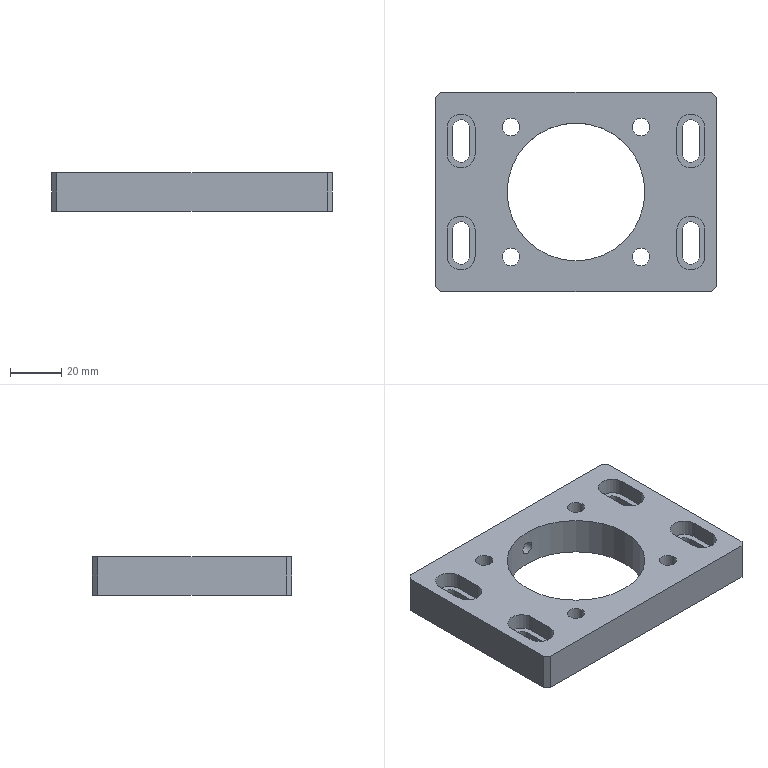Part | 1 solid | 52 faces | box 110 x 78 x 15 mm | volume 83115 mm3 | plane 30 | cylinder 22 | commonest cylinder face diameters 6.6 x8 11 x8 6.8 x4 5 x1 54 x1
STEP:
#1=CARTESIAN_POINT('',(-53.,39.,7.5));
#2=VERTEX_POINT('',#1);
#3=CARTESIAN_POINT('',(-55.,37.,7.5));
#4=VERTEX_POINT('',#3);
#5=CARTESIAN_POINT('',(-46.,46.,7.5));
#6=DIRECTION('',(-0.7071,-0.7071,0.));
#7=VECTOR('',#6,1000.);
#8=LINE('',#5,#7);
#9=EDGE_CURVE('',#2,#4,#8,.T.);
#10=ORIENTED_EDGE('',*,*,#9,.F.);
#11=CARTESIAN_POINT('',(-53.,39.,-7.5));
#12=VERTEX_POINT('',#11);
#13=CARTESIAN_POINT('',(-53.,39.,7.5));
#14=DIRECTION('',(0.,0.,1.));
#15=VECTOR('',#14,1000.);
#16=LINE('',#13,#15);
#17=EDGE_CURVE('',#12,#2,#16,.T.);
#18=ORIENTED_EDGE('',*,*,#17,.F.);
#19=CARTESIAN_POINT('',(-55.,37.,-7.5));
#20=VERTEX_POINT('',#19);
#21=CARTESIAN_POINT('',(-55.,37.,-7.5));
#22=DIRECTION('',(0.7071,0.7071,0.));
#23=VECTOR('',#22,1000.);
#24=LINE('',#21,#23);
#25=EDGE_CURVE('',#20,#12,#24,.T.);
#26=ORIENTED_EDGE('',*,*,#25,.F.);
#27=CARTESIAN_POINT('',(-55.,37.,7.5));
#28=DIRECTION('',(0.,0.,-1.));
#29=VECTOR('',#28,1000.);
#30=LINE('',#27,#29);
#31=EDGE_CURVE('',#4,#20,#30,.T.);
#32=ORIENTED_EDGE('',*,*,#31,.F.);
#33=EDGE_LOOP('',(#10,#18,#26,#32));
#34=FACE_BOUND('',#33,.T.);
#35=CARTESIAN_POINT('',(-55.,37.,7.5));
#36=DIRECTION('',(0.7071,-0.7071,0.));
#37=DIRECTION('',(0.,0.,-1.));
#38=AXIS2_PLACEMENT_3D('',#35,#36,#37);
#39=PLANE('',#38);
#40=ADVANCED_FACE('',(#34),#39,.F.);
#41=CARTESIAN_POINT('',(55.,37.,7.5));
#42=VERTEX_POINT('',#41);
#43=CARTESIAN_POINT('',(53.,39.,7.5));
#44=VERTEX_POINT('',#43);
#45=CARTESIAN_POINT('',(46.,46.,7.5));
#46=DIRECTION('',(-0.7071,0.7071,0.));
#47=VECTOR('',#46,1000.);
#48=LINE('',#45,#47);
#49=EDGE_CURVE('',#42,#44,#48,.T.);
#50=ORIENTED_EDGE('',*,*,#49,.F.);
#51=CARTESIAN_POINT('',(55.,37.,-7.5));
#52=VERTEX_POINT('',#51);
#53=CARTESIAN_POINT('',(55.,37.,7.5));
#54=DIRECTION('',(0.,0.,1.));
#55=VECTOR('',#54,1000.);
#56=LINE('',#53,#55);
#57=EDGE_CURVE('',#52,#42,#56,.T.);
#58=ORIENTED_EDGE('',*,*,#57,.F.);
#59=CARTESIAN_POINT('',(53.,39.,-7.5));
#60=VERTEX_POINT('',#59);
#61=CARTESIAN_POINT('',(53.,39.,-7.5));
#62=DIRECTION('',(0.7071,-0.7071,0.));
#63=VECTOR('',#62,1000.);
#64=LINE('',#61,#63);
#65=EDGE_CURVE('',#60,#52,#64,.T.);
#66=ORIENTED_EDGE('',*,*,#65,.F.);
#67=CARTESIAN_POINT('',(53.,39.,7.5));
#68=DIRECTION('',(0.,0.,-1.));
#69=VECTOR('',#68,1000.);
#70=LINE('',#67,#69);
#71=EDGE_CURVE('',#44,#60,#70,.T.);
#72=ORIENTED_EDGE('',*,*,#71,.F.);
#73=EDGE_LOOP('',(#50,#58,#66,#72));
#74=FACE_BOUND('',#73,.T.);
#75=CARTESIAN_POINT('',(53.,39.,7.5));
#76=DIRECTION('',(-0.7071,-0.7071,0.));
#77=DIRECTION('',(0.,0.,-1.));
#78=AXIS2_PLACEMENT_3D('',#75,#76,#77);
#79=PLANE('',#78);
#80=ADVANCED_FACE('',(#74),#79,.F.);
#81=CARTESIAN_POINT('',(53.,-39.,7.5));
#82=VERTEX_POINT('',#81);
#83=CARTESIAN_POINT('',(55.,-37.,7.5));
#84=VERTEX_POINT('',#83);
#85=CARTESIAN_POINT('',(46.,-46.,7.5));
#86=DIRECTION('',(0.7071,0.7071,0.));
#87=VECTOR('',#86,1000.);
#88=LINE('',#85,#87);
#89=EDGE_CURVE('',#82,#84,#88,.T.);
#90=ORIENTED_EDGE('',*,*,#89,.F.);
#91=CARTESIAN_POINT('',(53.,-39.,-7.5));
#92=VERTEX_POINT('',#91);
#93=CARTESIAN_POINT('',(53.,-39.,7.5));
#94=DIRECTION('',(0.,0.,1.));
#95=VECTOR('',#94,1000.);
#96=LINE('',#93,#95);
#97=EDGE_CURVE('',#92,#82,#96,.T.);
#98=ORIENTED_EDGE('',*,*,#97,.F.);
#99=CARTESIAN_POINT('',(55.,-37.,-7.5));
#100=VERTEX_POINT('',#99);
#101=CARTESIAN_POINT('',(55.,-37.,-7.5));
#102=DIRECTION('',(-0.7071,-0.7071,0.));
#103=VECTOR('',#102,1000.);
#104=LINE('',#101,#103);
#105=EDGE_CURVE('',#100,#92,#104,.T.);
#106=ORIENTED_EDGE('',*,*,#105,.F.);
#107=CARTESIAN_POINT('',(55.,-37.,7.5));
#108=DIRECTION('',(0.,0.,-1.));
#109=VECTOR('',#108,1000.);
#110=LINE('',#107,#109);
#111=EDGE_CURVE('',#84,#100,#110,.T.);
#112=ORIENTED_EDGE('',*,*,#111,.F.);
#113=EDGE_LOOP('',(#90,#98,#106,#112));
#114=FACE_BOUND('',#113,.T.);
#115=CARTESIAN_POINT('',(55.,-37.,7.5));
#116=DIRECTION('',(-0.7071,0.7071,0.));
#117=DIRECTION('',(0.,0.,-1.));
#118=AXIS2_PLACEMENT_3D('',#115,#116,#117);
#119=PLANE('',#118);
#120=ADVANCED_FACE('',(#114),#119,.F.);
#121=CARTESIAN_POINT('',(-55.,-37.,7.5));
#122=VERTEX_POINT('',#121);
#123=CARTESIAN_POINT('',(-53.,-39.,7.5));
#124=VERTEX_POINT('',#123);
#125=CARTESIAN_POINT('',(-46.,-46.,7.5));
#126=DIRECTION('',(0.7071,-0.7071,0.));
#127=VECTOR('',#126,1000.);
#128=LINE('',#125,#127);
#129=EDGE_CURVE('',#122,#124,#128,.T.);
#130=ORIENTED_EDGE('',*,*,#129,.F.);
#131=CARTESIAN_POINT('',(-55.,-37.,-7.5));
#132=VERTEX_POINT('',#131);
#133=CARTESIAN_POINT('',(-55.,-37.,7.5));
#134=DIRECTION('',(0.,0.,1.));
#135=VECTOR('',#134,1000.);
#136=LINE('',#133,#135);
#137=EDGE_CURVE('',#132,#122,#136,.T.);
#138=ORIENTED_EDGE('',*,*,#137,.F.);
#139=CARTESIAN_POINT('',(-53.,-39.,-7.5));
#140=VERTEX_POINT('',#139);
#141=CARTESIAN_POINT('',(-53.,-39.,-7.5));
#142=DIRECTION('',(-0.7071,0.7071,0.));
#143=VECTOR('',#142,1000.);
#144=LINE('',#141,#143);
#145=EDGE_CURVE('',#140,#132,#144,.T.);
#146=ORIENTED_EDGE('',*,*,#145,.F.);
#147=CARTESIAN_POINT('',(-53.,-39.,7.5));
#148=DIRECTION('',(0.,0.,-1.));
#149=VECTOR('',#148,1000.);
#150=LINE('',#147,#149);
#151=EDGE_CURVE('',#124,#140,#150,.T.);
#152=ORIENTED_EDGE('',*,*,#151,.F.);
#153=EDGE_LOOP('',(#130,#138,#146,#152));
#154=FACE_BOUND('',#153,.T.);
#155=CARTESIAN_POINT('',(-53.,-39.,7.5));
#156=DIRECTION('',(0.7071,0.7071,0.));
#157=DIRECTION('',(0.,0.,-1.));
#158=AXIS2_PLACEMENT_3D('',#155,#156,#157);
#159=PLANE('',#158);
#160=ADVANCED_FACE('',(#154),#159,.F.);
#161=CARTESIAN_POINT('',(50.5,25.,7.5));
#162=VERTEX_POINT('',#161);
#163=CARTESIAN_POINT('',(50.5,25.,1.1));
#164=VERTEX_POINT('',#163);
#165=CARTESIAN_POINT('',(50.5,25.,1.1));
#166=DIRECTION('',(0.,0.,-1.));
#167=VECTOR('',#166,1000.);
#168=LINE('',#165,#167);
#169=EDGE_CURVE('',#162,#164,#168,.T.);
#170=ORIENTED_EDGE('',*,*,#169,.T.);
#171=CARTESIAN_POINT('',(50.5,15.,1.1));
#172=VERTEX_POINT('',#171);
#173=CARTESIAN_POINT('',(50.5,15.,1.1));
#174=DIRECTION('',(0.,1.,0.));
#175=VECTOR('',#174,1000.);
#176=LINE('',#173,#175);
#177=EDGE_CURVE('',#172,#164,#176,.T.);
#178=ORIENTED_EDGE('',*,*,#177,.F.);
#179=CARTESIAN_POINT('',(50.5,15.,7.5));
#180=VERTEX_POINT('',#179);
#181=CARTESIAN_POINT('',(50.5,15.,1.1));
#182=DIRECTION('',(0.,0.,-1.));
#183=VECTOR('',#182,1000.);
#184=LINE('',#181,#183);
#185=EDGE_CURVE('',#180,#172,#184,.T.);
#186=ORIENTED_EDGE('',*,*,#185,.F.);
#187=CARTESIAN_POINT('',(50.5,15.,7.5));
#188=DIRECTION('',(0.,1.,0.));
#189=VECTOR('',#188,1000.);
#190=LINE('',#187,#189);
#191=EDGE_CURVE('',#180,#162,#190,.T.);
#192=ORIENTED_EDGE('',*,*,#191,.T.);
#193=EDGE_LOOP('',(#170,#178,#186,#192));
#194=FACE_BOUND('',#193,.T.);
#195=CARTESIAN_POINT('',(50.5,15.,1.1));
#196=DIRECTION('',(1.,0.,0.));
#197=DIRECTION('',(0.,0.,-1.));
#198=AXIS2_PLACEMENT_3D('',#195,#196,#197);
#199=PLANE('',#198);
#200=ADVANCED_FACE('',(#194),#199,.F.);
#201=CARTESIAN_POINT('',(48.3,25.,1.1));
#202=VERTEX_POINT('',#201);
#203=CARTESIAN_POINT('',(48.3,25.,-7.5));
#204=VERTEX_POINT('',#203);
#205=CARTESIAN_POINT('',(48.3,25.,-7.5));
#206=DIRECTION('',(0.,0.,-1.));
#207=VECTOR('',#206,1000.);
#208=LINE('',#205,#207);
#209=EDGE_CURVE('',#202,#204,#208,.T.);
#210=ORIENTED_EDGE('',*,*,#209,.T.);
#211=CARTESIAN_POINT('',(48.3,15.,-7.5));
#212=VERTEX_POINT('',#211);
#213=CARTESIAN_POINT('',(48.3,15.,-7.5));
#214=DIRECTION('',(0.,1.,0.));
#215=VECTOR('',#214,1000.);
#216=LINE('',#213,#215);
#217=EDGE_CURVE('',#212,#204,#216,.T.);
#218=ORIENTED_EDGE('',*,*,#217,.F.);
#219=CARTESIAN_POINT('',(48.3,15.,1.1));
#220=VERTEX_POINT('',#219);
#221=CARTESIAN_POINT('',(48.3,15.,-7.5));
#222=DIRECTION('',(0.,0.,-1.));
#223=VECTOR('',#222,1000.);
#224=LINE('',#221,#223);
#225=EDGE_CURVE('',#220,#212,#224,.T.);
#226=ORIENTED_EDGE('',*,*,#225,.F.);
#227=CARTESIAN_POINT('',(48.3,15.,1.1));
#228=DIRECTION('',(0.,1.,0.));
#229=VECTOR('',#228,1000.);
#230=LINE('',#227,#229);
#231=EDGE_CURVE('',#220,#202,#230,.T.);
#232=ORIENTED_EDGE('',*,*,#231,.T.);
#233=EDGE_LOOP('',(#210,#218,#226,#232));
#234=FACE_BOUND('',#233,.T.);
#235=CARTESIAN_POINT('',(48.3,15.,-7.5));
#236=DIRECTION('',(1.,0.,0.));
#237=DIRECTION('',(0.,0.,-1.));
#238=AXIS2_PLACEMENT_3D('',#235,#236,#237);
#239=PLANE('',#238);
#240=ADVANCED_FACE('',(#234),#239,.F.);
#241=CARTESIAN_POINT('',(41.7,25.,-7.5));
#242=VERTEX_POINT('',#241);
#243=CARTESIAN_POINT('',(41.7,25.,1.1));
#244=VERTEX_POINT('',#243);
#245=CARTESIAN_POINT('',(41.7,25.,7.5));
#246=DIRECTION('',(0.,0.,1.));
#247=VECTOR('',#246,1000.);
#248=LINE('',#245,#247);
#249=EDGE_CURVE('',#242,#244,#248,.T.);
#250=ORIENTED_EDGE('',*,*,#249,.T.);
#251=CARTESIAN_POINT('',(41.7,15.,1.1));
#252=VERTEX_POINT('',#251);
#253=CARTESIAN_POINT('',(41.7,15.,1.1));
#254=DIRECTION('',(0.,1.,0.));
#255=VECTOR('',#254,1000.);
#256=LINE('',#253,#255);
#257=EDGE_CURVE('',#252,#244,#256,.T.);
#258=ORIENTED_EDGE('',*,*,#257,.F.);
#259=CARTESIAN_POINT('',(41.7,15.,-7.5));
#260=VERTEX_POINT('',#259);
#261=CARTESIAN_POINT('',(41.7,15.,7.5));
#262=DIRECTION('',(0.,0.,-1.));
#263=VECTOR('',#262,1000.);
#264=LINE('',#261,#263);
#265=EDGE_CURVE('',#252,#260,#264,.T.);
#266=ORIENTED_EDGE('',*,*,#265,.T.);
#267=CARTESIAN_POINT('',(41.7,15.,-7.5));
#268=DIRECTION('',(0.,1.,0.));
#269=VECTOR('',#268,1000.);
#270=LINE('',#267,#269);
#271=EDGE_CURVE('',#260,#242,#270,.T.);
#272=ORIENTED_EDGE('',*,*,#271,.T.);
#273=EDGE_LOOP('',(#250,#258,#266,#272));
#274=FACE_BOUND('',#273,.T.);
#275=CARTESIAN_POINT('',(41.7,15.,7.5));
#276=DIRECTION('',(-1.,0.,0.));
#277=DIRECTION('',(0.,0.,1.));
#278=AXIS2_PLACEMENT_3D('',#275,#276,#277);
#279=PLANE('',#278);
#280=ADVANCED_FACE('',(#274),#279,.F.);
#281=CARTESIAN_POINT('',(39.5,25.,1.1));
#282=VERTEX_POINT('',#281);
#283=CARTESIAN_POINT('',(39.5,25.,7.5));
#284=VERTEX_POINT('',#283);
#285=CARTESIAN_POINT('',(39.5,25.,7.5));
#286=DIRECTION('',(0.,0.,1.));
#287=VECTOR('',#286,1000.);
#288=LINE('',#285,#287);
#289=EDGE_CURVE('',#282,#284,#288,.T.);
#290=ORIENTED_EDGE('',*,*,#289,.T.);
#291=CARTESIAN_POINT('',(39.5,15.,7.5));
#292=VERTEX_POINT('',#291);
#293=CARTESIAN_POINT('',(39.5,15.,7.5));
#294=DIRECTION('',(0.,1.,0.));
#295=VECTOR('',#294,1000.);
#296=LINE('',#293,#295);
#297=EDGE_CURVE('',#292,#284,#296,.T.);
#298=ORIENTED_EDGE('',*,*,#297,.F.);
#299=CARTESIAN_POINT('',(39.5,15.,1.1));
#300=VERTEX_POINT('',#299);
#301=CARTESIAN_POINT('',(39.5,15.,7.5));
#302=DIRECTION('',(0.,0.,-1.));
#303=VECTOR('',#302,1000.);
#304=LINE('',#301,#303);
#305=EDGE_CURVE('',#292,#300,#304,.T.);
#306=ORIENTED_EDGE('',*,*,#305,.T.);
#307=CARTESIAN_POINT('',(39.5,15.,1.1));
#308=DIRECTION('',(0.,1.,0.));
#309=VECTOR('',#308,1000.);
#310=LINE('',#307,#309);
#311=EDGE_CURVE('',#300,#282,#310,.T.);
#312=ORIENTED_EDGE('',*,*,#311,.T.);
#313=EDGE_LOOP('',(#290,#298,#306,#312));
#314=FACE_BOUND('',#313,.T.);
#315=CARTESIAN_POINT('',(39.5,15.,7.5));
#316=DIRECTION('',(-1.,0.,0.));
#317=DIRECTION('',(0.,0.,1.));
#318=AXIS2_PLACEMENT_3D('',#315,#316,#317);
#319=PLANE('',#318);
#320=ADVANCED_FACE('',(#314),#319,.F.);
#321=CARTESIAN_POINT('',(45.,15.,7.5));
#322=DIRECTION('',(0.,0.,1.));
#323=DIRECTION('',(1.,0.,0.));
#324=AXIS2_PLACEMENT_3D('',#321,#322,#323);
#325=CIRCLE('',#324,5.5);
#326=EDGE_CURVE('',#292,#180,#325,.T.);
#327=ORIENTED_EDGE('',*,*,#326,.T.);
#328=ORIENTED_EDGE('',*,*,#185,.T.);
#329=CARTESIAN_POINT('',(45.,15.,1.1));
#330=DIRECTION('',(0.,0.,1.));
#331=DIRECTION('',(1.,0.,0.));
#332=AXIS2_PLACEMENT_3D('',#329,#330,#331);
#333=CIRCLE('',#332,5.5);
#334=EDGE_CURVE('',#300,#172,#333,.T.);
#335=ORIENTED_EDGE('',*,*,#334,.F.);
#336=ORIENTED_EDGE('',*,*,#305,.F.);
#337=EDGE_LOOP('',(#327,#328,#335,#336));
#338=FACE_BOUND('',#337,.T.);
#339=CARTESIAN_POINT('',(45.,15.,7.5));
#340=DIRECTION('',(0.,0.,1.));
#341=DIRECTION('',(1.,0.,0.));
#342=AXIS2_PLACEMENT_3D('',#339,#340,#341);
#343=CYLINDRICAL_SURFACE('',#342,5.5);
#344=ADVANCED_FACE('',(#338),#343,.F.);
#345=CARTESIAN_POINT('',(45.,15.,1.1));
#346=DIRECTION('',(0.,0.,1.));
#347=DIRECTION('',(1.,0.,0.));
#348=AXIS2_PLACEMENT_3D('',#345,#346,#347);
#349=CIRCLE('',#348,3.3);
#350=EDGE_CURVE('',#252,#220,#349,.T.);
#351=ORIENTED_EDGE('',*,*,#350,.T.);
#352=ORIENTED_EDGE('',*,*,#225,.T.);
#353=CARTESIAN_POINT('',(45.,15.,-7.5));
#354=DIRECTION('',(0.,0.,1.));
#355=DIRECTION('',(1.,0.,0.));
#356=AXIS2_PLACEMENT_3D('',#353,#354,#355);
#357=CIRCLE('',#356,3.3);
#358=EDGE_CURVE('',#260,#212,#357,.T.);
#359=ORIENTED_EDGE('',*,*,#358,.F.);
#360=ORIENTED_EDGE('',*,*,#265,.F.);
#361=EDGE_LOOP('',(#351,#352,#359,#360));
#362=FACE_BOUND('',#361,.T.);
#363=CARTESIAN_POINT('',(45.,15.,7.5));
#364=DIRECTION('',(0.,0.,1.));
#365=DIRECTION('',(1.,0.,0.));
#366=AXIS2_PLACEMENT_3D('',#363,#364,#365);
#367=CYLINDRICAL_SURFACE('',#366,3.3);
#368=ADVANCED_FACE('',(#362),#367,.F.);
#369=CARTESIAN_POINT('',(45.,25.,1.1));
#370=DIRECTION('',(0.,0.,1.));
#371=DIRECTION('',(1.,0.,0.));
#372=AXIS2_PLACEMENT_3D('',#369,#370,#371);
#373=CIRCLE('',#372,5.5);
#374=EDGE_CURVE('',#164,#282,#373,.T.);
#375=ORIENTED_EDGE('',*,*,#374,.F.);
#376=ORIENTED_EDGE('',*,*,#169,.F.);
#377=CARTESIAN_POINT('',(45.,25.,7.5));
#378=DIRECTION('',(0.,0.,1.));
#379=DIRECTION('',(1.,0.,0.));
#380=AXIS2_PLACEMENT_3D('',#377,#378,#379);
#381=CIRCLE('',#380,5.5);
#382=EDGE_CURVE('',#162,#284,#381,.T.);
#383=ORIENTED_EDGE('',*,*,#382,.T.);
#384=ORIENTED_EDGE('',*,*,#289,.F.);
#385=EDGE_LOOP('',(#375,#376,#383,#384));
#386=FACE_BOUND('',#385,.T.);
#387=CARTESIAN_POINT('',(45.,25.,7.5));
#388=DIRECTION('',(0.,0.,1.));
#389=DIRECTION('',(1.,0.,0.));
#390=AXIS2_PLACEMENT_3D('',#387,#388,#389);
#391=CYLINDRICAL_SURFACE('',#390,5.5);
#392=ADVANCED_FACE('',(#386),#391,.F.);
#393=CARTESIAN_POINT('',(45.,25.,1.1));
#394=DIRECTION('',(0.,0.,1.));
#395=DIRECTION('',(1.,0.,0.));
#396=AXIS2_PLACEMENT_3D('',#393,#394,#395);
#397=CIRCLE('',#396,3.3);
#398=EDGE_CURVE('',#202,#244,#397,.T.);
#399=ORIENTED_EDGE('',*,*,#398,.F.);
#400=ORIENTED_EDGE('',*,*,#231,.F.);
#401=ORIENTED_EDGE('',*,*,#350,.F.);
#402=ORIENTED_EDGE('',*,*,#257,.T.);
#403=EDGE_LOOP('',(#399,#400,#401,#402));
#404=FACE_BOUND('',#403,.T.);
#405=ORIENTED_EDGE('',*,*,#311,.F.);
#406=ORIENTED_EDGE('',*,*,#334,.T.);
#407=ORIENTED_EDGE('',*,*,#177,.T.);
#408=ORIENTED_EDGE('',*,*,#374,.T.);
#409=EDGE_LOOP('',(#405,#406,#407,#408));
#410=FACE_BOUND('',#409,.T.);
#411=CARTESIAN_POINT('',(48.3,25.,1.1));
#412=DIRECTION('',(0.,0.,-1.));
#413=DIRECTION('',(-1.,0.,0.));
#414=AXIS2_PLACEMENT_3D('',#411,#412,#413);
#415=PLANE('',#414);
#416=ADVANCED_FACE('',(#404,#410),#415,.F.);
#417=CARTESIAN_POINT('',(45.,25.,-7.5));
#418=DIRECTION('',(0.,0.,1.));
#419=DIRECTION('',(1.,0.,0.));
#420=AXIS2_PLACEMENT_3D('',#417,#418,#419);
#421=CIRCLE('',#420,3.3);
#422=EDGE_CURVE('',#204,#242,#421,.T.);
#423=ORIENTED_EDGE('',*,*,#422,.F.);
#424=ORIENTED_EDGE('',*,*,#209,.F.);
#425=ORIENTED_EDGE('',*,*,#398,.T.);
#426=ORIENTED_EDGE('',*,*,#249,.F.);
#427=EDGE_LOOP('',(#423,#424,#425,#426));
#428=FACE_BOUND('',#427,.T.);
#429=CARTESIAN_POINT('',(45.,25.,7.5));
#430=DIRECTION('',(0.,0.,1.));
#431=DIRECTION('',(1.,0.,0.));
#432=AXIS2_PLACEMENT_3D('',#429,#430,#431);
#433=CYLINDRICAL_SURFACE('',#432,3.3);
#434=ADVANCED_FACE('',(#428),#433,.F.);
#435=CARTESIAN_POINT('',(-39.5,25.,7.5));
#436=VERTEX_POINT('',#435);
#437=CARTESIAN_POINT('',(-39.5,25.,1.1));
#438=VERTEX_POINT('',#437);
#439=CARTESIAN_POINT('',(-39.5,25.,1.1));
#440=DIRECTION('',(0.,0.,-1.));
#441=VECTOR('',#440,1000.);
#442=LINE('',#439,#441);
#443=EDGE_CURVE('',#436,#438,#442,.T.);
#444=ORIENTED_EDGE('',*,*,#443,.T.);
#445=CARTESIAN_POINT('',(-39.5,15.,1.1));
#446=VERTEX_POINT('',#445);
#447=CARTESIAN_POINT('',(-39.5,25.,1.1));
#448=DIRECTION('',(0.,1.,0.));
#449=VECTOR('',#448,1000.);
#450=LINE('',#447,#449);
#451=EDGE_CURVE('',#446,#438,#450,.T.);
#452=ORIENTED_EDGE('',*,*,#451,.F.);
#453=CARTESIAN_POINT('',(-39.5,15.,7.5));
#454=VERTEX_POINT('',#453);
#455=CARTESIAN_POINT('',(-39.5,15.,1.1));
#456=DIRECTION('',(0.,0.,-1.));
#457=VECTOR('',#456,1000.);
#458=LINE('',#455,#457);
#459=EDGE_CURVE('',#454,#446,#458,.T.);
#460=ORIENTED_EDGE('',*,*,#459,.F.);
#461=CARTESIAN_POINT('',(-39.5,15.,7.5));
#462=DIRECTION('',(0.,1.,0.));
#463=VECTOR('',#462,1000.);
#464=LINE('',#461,#463);
#465=EDGE_CURVE('',#454,#436,#464,.T.);
#466=ORIENTED_EDGE('',*,*,#465,.T.);
#467=EDGE_LOOP('',(#444,#452,#460,#466));
#468=FACE_BOUND('',#467,.T.);
#469=CARTESIAN_POINT('',(-39.5,15.,1.1));
#470=DIRECTION('',(1.,0.,0.));
#471=DIRECTION('',(0.,0.,-1.));
#472=AXIS2_PLACEMENT_3D('',#469,#470,#471);
#473=PLANE('',#472);
#474=ADVANCED_FACE('',(#468),#473,.F.);
#475=CARTESIAN_POINT('',(-41.7,25.,1.1));
#476=VERTEX_POINT('',#475);
#477=CARTESIAN_POINT('',(-41.7,25.,-7.5));
#478=VERTEX_POINT('',#477);
#479=CARTESIAN_POINT('',(-41.7,25.,-7.5));
#480=DIRECTION('',(0.,0.,-1.));
#481=VECTOR('',#480,1000.);
#482=LINE('',#479,#481);
#483=EDGE_CURVE('',#476,#478,#482,.T.);
#484=ORIENTED_EDGE('',*,*,#483,.T.);
#485=CARTESIAN_POINT('',(-41.7,15.,-7.5));
#486=VERTEX_POINT('',#485);
#487=CARTESIAN_POINT('',(-41.7,15.,-7.5));
#488=DIRECTION('',(0.,1.,0.));
#489=VECTOR('',#488,1000.);
#490=LINE('',#487,#489);
#491=EDGE_CURVE('',#486,#478,#490,.T.);
#492=ORIENTED_EDGE('',*,*,#491,.F.);
#493=CARTESIAN_POINT('',(-41.7,15.,1.1));
#494=VERTEX_POINT('',#493);
#495=CARTESIAN_POINT('',(-41.7,15.,-7.5));
#496=DIRECTION('',(0.,0.,-1.));
#497=VECTOR('',#496,1000.);
#498=LINE('',#495,#497);
#499=EDGE_CURVE('',#494,#486,#498,.T.);
#500=ORIENTED_EDGE('',*,*,#499,.F.);
#501=CARTESIAN_POINT('',(-41.7,15.,1.1));
#502=DIRECTION('',(0.,1.,0.));
#503=VECTOR('',#502,1000.);
#504=LINE('',#501,#503);
#505=EDGE_CURVE('',#494,#476,#504,.T.);
#506=ORIENTED_EDGE('',*,*,#505,.T.);
#507=EDGE_LOOP('',(#484,#492,#500,#506));
#508=FACE_BOUND('',#507,.T.);
#509=CARTESIAN_POINT('',(-41.7,15.,-7.5));
#510=DIRECTION('',(1.,0.,0.));
#511=DIRECTION('',(0.,0.,-1.));
#512=AXIS2_PLACEMENT_3D('',#509,#510,#511);
#513=PLANE('',#512);
#514=ADVANCED_FACE('',(#508),#513,.F.);
#515=CARTESIAN_POINT('',(-48.3,25.,-7.5));
#516=VERTEX_POINT('',#515);
#517=CARTESIAN_POINT('',(-48.3,25.,1.1));
#518=VERTEX_POINT('',#517);
#519=CARTESIAN_POINT('',(-48.3,25.,7.5));
#520=DIRECTION('',(0.,0.,1.));
#521=VECTOR('',#520,1000.);
#522=LINE('',#519,#521);
#523=EDGE_CURVE('',#516,#518,#522,.T.);
#524=ORIENTED_EDGE('',*,*,#523,.T.);
#525=CARTESIAN_POINT('',(-48.3,15.,1.1));
#526=VERTEX_POINT('',#525);
#527=CARTESIAN_POINT('',(-48.3,25.,1.1));
#528=DIRECTION('',(0.,1.,0.));
#529=VECTOR('',#528,1000.);
#530=LINE('',#527,#529);
#531=EDGE_CURVE('',#526,#518,#530,.T.);
#532=ORIENTED_EDGE('',*,*,#531,.F.);
#533=CARTESIAN_POINT('',(-48.3,15.,-7.5));
#534=VERTEX_POINT('',#533);
#535=CARTESIAN_POINT('',(-48.3,15.,7.5));
#536=DIRECTION('',(0.,0.,-1.));
#537=VECTOR('',#536,1000.);
#538=LINE('',#535,#537);
#539=EDGE_CURVE('',#526,#534,#538,.T.);
#540=ORIENTED_EDGE('',*,*,#539,.T.);
#541=CARTESIAN_POINT('',(-48.3,15.,-7.5));
#542=DIRECTION('',(0.,1.,0.));
#543=VECTOR('',#542,1000.);
#544=LINE('',#541,#543);
#545=EDGE_CURVE('',#534,#516,#544,.T.);
#546=ORIENTED_EDGE('',*,*,#545,.T.);
#547=EDGE_LOOP('',(#524,#532,#540,#546));
#548=FACE_BOUND('',#547,.T.);
#549=CARTESIAN_POINT('',(-48.3,15.,7.5));
#550=DIRECTION('',(-1.,0.,0.));
#551=DIRECTION('',(0.,0.,1.));
#552=AXIS2_PLACEMENT_3D('',#549,#550,#551);
#553=PLANE('',#552);
#554=ADVANCED_FACE('',(#548),#553,.F.);
#555=CARTESIAN_POINT('',(-50.5,25.,1.1));
#556=VERTEX_POINT('',#555);
#557=CARTESIAN_POINT('',(-50.5,25.,7.5));
#558=VERTEX_POINT('',#557);
#559=CARTESIAN_POINT('',(-50.5,25.,7.5));
#560=DIRECTION('',(0.,0.,1.));
#561=VECTOR('',#560,1000.);
#562=LINE('',#559,#561);
#563=EDGE_CURVE('',#556,#558,#562,.T.);
#564=ORIENTED_EDGE('',*,*,#563,.T.);
#565=CARTESIAN_POINT('',(-50.5,15.,7.5));
#566=VERTEX_POINT('',#565);
#567=CARTESIAN_POINT('',(-50.5,15.,7.5));
#568=DIRECTION('',(0.,1.,0.));
#569=VECTOR('',#568,1000.);
#570=LINE('',#567,#569);
#571=EDGE_CURVE('',#566,#558,#570,.T.);
#572=ORIENTED_EDGE('',*,*,#571,.F.);
#573=CARTESIAN_POINT('',(-50.5,15.,1.1));
#574=VERTEX_POINT('',#573);
#575=CARTESIAN_POINT('',(-50.5,15.,7.5));
#576=DIRECTION('',(0.,0.,-1.));
#577=VECTOR('',#576,1000.);
#578=LINE('',#575,#577);
#579=EDGE_CURVE('',#566,#574,#578,.T.);
#580=ORIENTED_EDGE('',*,*,#579,.T.);
#581=CARTESIAN_POINT('',(-50.5,15.,1.1));
#582=DIRECTION('',(0.,1.,0.));
#583=VECTOR('',#582,1000.);
#584=LINE('',#581,#583);
#585=EDGE_CURVE('',#574,#556,#584,.T.);
#586=ORIENTED_EDGE('',*,*,#585,.T.);
#587=EDGE_LOOP('',(#564,#572,#580,#586));
#588=FACE_BOUND('',#587,.T.);
#589=CARTESIAN_POINT('',(-50.5,15.,7.5));
#590=DIRECTION('',(-1.,0.,0.));
#591=DIRECTION('',(0.,0.,1.));
#592=AXIS2_PLACEMENT_3D('',#589,#590,#591);
#593=PLANE('',#592);
#594=ADVANCED_FACE('',(#588),#593,.F.);
#595=CARTESIAN_POINT('',(-45.,15.,7.5));
#596=DIRECTION('',(0.,0.,1.));
#597=DIRECTION('',(1.,0.,0.));
#598=AXIS2_PLACEMENT_3D('',#595,#596,#597);
#599=CIRCLE('',#598,5.5);
#600=EDGE_CURVE('',#566,#454,#599,.T.);
#601=ORIENTED_EDGE('',*,*,#600,.T.);
#602=ORIENTED_EDGE('',*,*,#459,.T.);
#603=CARTESIAN_POINT('',(-45.,15.,1.1));
#604=DIRECTION('',(0.,0.,1.));
#605=DIRECTION('',(-1.,0.,0.));
#606=AXIS2_PLACEMENT_3D('',#603,#604,#605);
#607=CIRCLE('',#606,5.5);
#608=EDGE_CURVE('',#574,#446,#607,.T.);
#609=ORIENTED_EDGE('',*,*,#608,.F.);
#610=ORIENTED_EDGE('',*,*,#579,.F.);
#611=EDGE_LOOP('',(#601,#602,#609,#610));
#612=FACE_BOUND('',#611,.T.);
#613=CARTESIAN_POINT('',(-45.,15.,7.5));
#614=DIRECTION('',(0.,0.,1.));
#615=DIRECTION('',(1.,0.,0.));
#616=AXIS2_PLACEMENT_3D('',#613,#614,#615);
#617=CYLINDRICAL_SURFACE('',#616,5.5);
#618=ADVANCED_FACE('',(#612),#617,.F.);
#619=CARTESIAN_POINT('',(-45.,15.,1.1));
#620=DIRECTION('',(0.,0.,1.));
#621=DIRECTION('',(-1.,0.,0.));
#622=AXIS2_PLACEMENT_3D('',#619,#620,#621);
#623=CIRCLE('',#622,3.3);
#624=EDGE_CURVE('',#526,#494,#623,.T.);
#625=ORIENTED_EDGE('',*,*,#624,.T.);
#626=ORIENTED_EDGE('',*,*,#499,.T.);
#627=CARTESIAN_POINT('',(-45.,15.,-7.5));
#628=DIRECTION('',(0.,0.,1.));
#629=DIRECTION('',(1.,0.,0.));
#630=AXIS2_PLACEMENT_3D('',#627,#628,#629);
#631=CIRCLE('',#630,3.3);
#632=EDGE_CURVE('',#534,#486,#631,.T.);
#633=ORIENTED_EDGE('',*,*,#632,.F.);
#634=ORIENTED_EDGE('',*,*,#539,.F.);
#635=EDGE_LOOP('',(#625,#626,#633,#634));
#636=FACE_BOUND('',#635,.T.);
#637=CARTESIAN_POINT('',(-45.,15.,7.5));
#638=DIRECTION('',(0.,0.,1.));
#639=DIRECTION('',(1.,0.,0.));
#640=AXIS2_PLACEMENT_3D('',#637,#638,#639);
#641=CYLINDRICAL_SURFACE('',#640,3.3);
#642=ADVANCED_FACE('',(#636),#641,.F.);
#643=CARTESIAN_POINT('',(-45.,25.,1.1));
#644=DIRECTION('',(0.,0.,1.));
#645=DIRECTION('',(-1.,0.,0.));
#646=AXIS2_PLACEMENT_3D('',#643,#644,#645);
#647=CIRCLE('',#646,5.5);
#648=EDGE_CURVE('',#438,#556,#647,.T.);
#649=ORIENTED_EDGE('',*,*,#648,.F.);
#650=ORIENTED_EDGE('',*,*,#443,.F.);
#651=CARTESIAN_POINT('',(-45.,25.,7.5));
#652=DIRECTION('',(0.,0.,1.));
#653=DIRECTION('',(1.,0.,0.));
#654=AXIS2_PLACEMENT_3D('',#651,#652,#653);
#655=CIRCLE('',#654,5.5);
#656=EDGE_CURVE('',#436,#558,#655,.T.);
#657=ORIENTED_EDGE('',*,*,#656,.T.);
#658=ORIENTED_EDGE('',*,*,#563,.F.);
#659=EDGE_LOOP('',(#649,#650,#657,#658));
#660=FACE_BOUND('',#659,.T.);
#661=CARTESIAN_POINT('',(-45.,25.,7.5));
#662=DIRECTION('',(0.,0.,1.));
#663=DIRECTION('',(1.,0.,0.));
#664=AXIS2_PLACEMENT_3D('',#661,#662,#663);
#665=CYLINDRICAL_SURFACE('',#664,5.5);
#666=ADVANCED_FACE('',(#660),#665,.F.);
#667=CARTESIAN_POINT('',(-45.,25.,1.1));
#668=DIRECTION('',(0.,0.,1.));
#669=DIRECTION('',(-1.,0.,0.));
#670=AXIS2_PLACEMENT_3D('',#667,#668,#669);
#671=CIRCLE('',#670,3.3);
#672=EDGE_CURVE('',#476,#518,#671,.T.);
#673=ORIENTED_EDGE('',*,*,#672,.F.);
#674=ORIENTED_EDGE('',*,*,#505,.F.);
#675=ORIENTED_EDGE('',*,*,#624,.F.);
#676=ORIENTED_EDGE('',*,*,#531,.T.);
#677=EDGE_LOOP('',(#673,#674,#675,#676));
#678=FACE_BOUND('',#677,.T.);
#679=ORIENTED_EDGE('',*,*,#585,.F.);
#680=ORIENTED_EDGE('',*,*,#608,.T.);
#681=ORIENTED_EDGE('',*,*,#451,.T.);
#682=ORIENTED_EDGE('',*,*,#648,.T.);
#683=EDGE_LOOP('',(#679,#680,#681,#682));
#684=FACE_BOUND('',#683,.T.);
#685=CARTESIAN_POINT('',(48.3,25.,1.1));
#686=DIRECTION('',(0.,0.,-1.));
#687=DIRECTION('',(-1.,0.,0.));
#688=AXIS2_PLACEMENT_3D('',#685,#686,#687);
#689=PLANE('',#688);
#690=ADVANCED_FACE('',(#678,#684),#689,.F.);
#691=CARTESIAN_POINT('',(-45.,25.,-7.5));
#692=DIRECTION('',(0.,0.,1.));
#693=DIRECTION('',(1.,0.,0.));
#694=AXIS2_PLACEMENT_3D('',#691,#692,#693);
#695=CIRCLE('',#694,3.3);
#696=EDGE_CURVE('',#478,#516,#695,.T.);
#697=ORIENTED_EDGE('',*,*,#696,.F.);
#698=ORIENTED_EDGE('',*,*,#483,.F.);
#699=ORIENTED_EDGE('',*,*,#672,.T.);
#700=ORIENTED_EDGE('',*,*,#523,.F.);
#701=EDGE_LOOP('',(#697,#698,#699,#700));
#702=FACE_BOUND('',#701,.T.);
#703=CARTESIAN_POINT('',(-45.,25.,7.5));
#704=DIRECTION('',(0.,0.,1.));
#705=DIRECTION('',(1.,0.,0.));
#706=AXIS2_PLACEMENT_3D('',#703,#704,#705);
#707=CYLINDRICAL_SURFACE('',#706,3.3);
#708=ADVANCED_FACE('',(#702),#707,.F.);
#709=CARTESIAN_POINT('',(-39.5,-15.,7.5));
#710=VERTEX_POINT('',#709);
#711=CARTESIAN_POINT('',(-39.5,-15.,1.1));
#712=VERTEX_POINT('',#711);
#713=CARTESIAN_POINT('',(-39.5,-15.,7.5));
#714=DIRECTION('',(0.,0.,-1.));
#715=VECTOR('',#714,1000.);
#716=LINE('',#713,#715);
#717=EDGE_CURVE('',#710,#712,#716,.T.);
#718=ORIENTED_EDGE('',*,*,#717,.T.);
#719=CARTESIAN_POINT('',(-39.5,-25.,1.1));
#720=VERTEX_POINT('',#719);
#721=CARTESIAN_POINT('',(-39.5,25.,1.1));
#722=DIRECTION('',(0.,1.,0.));
#723=VECTOR('',#722,1000.);
#724=LINE('',#721,#723);
#725=EDGE_CURVE('',#720,#712,#724,.T.);
#726=ORIENTED_EDGE('',*,*,#725,.F.);
#727=CARTESIAN_POINT('',(-39.5,-25.,7.5));
#728=VERTEX_POINT('',#727);
#729=CARTESIAN_POINT('',(-39.5,-25.,7.5));
#730=DIRECTION('',(0.,0.,-1.));
#731=VECTOR('',#730,1000.);
#732=LINE('',#729,#731);
#733=EDGE_CURVE('',#728,#720,#732,.T.);
#734=ORIENTED_EDGE('',*,*,#733,.F.);
#735=CARTESIAN_POINT('',(-39.5,15.,7.5));
#736=DIRECTION('',(0.,1.,0.));
#737=VECTOR('',#736,1000.);
#738=LINE('',#735,#737);
#739=EDGE_CURVE('',#728,#710,#738,.T.);
#740=ORIENTED_EDGE('',*,*,#739,.T.);
#741=EDGE_LOOP('',(#718,#726,#734,#740));
#742=FACE_BOUND('',#741,.T.);
#743=CARTESIAN_POINT('',(-39.5,15.,1.1));
#744=DIRECTION('',(1.,0.,0.));
#745=DIRECTION('',(0.,0.,-1.));
#746=AXIS2_PLACEMENT_3D('',#743,#744,#745);
#747=PLANE('',#746);
#748=ADVANCED_FACE('',(#742),#747,.F.);
#749=CARTESIAN_POINT('',(-41.7,-15.,1.1));
#750=VERTEX_POINT('',#749);
#751=CARTESIAN_POINT('',(-41.7,-15.,-7.5));
#752=VERTEX_POINT('',#751);
#753=CARTESIAN_POINT('',(-41.7,-15.,7.5));
#754=DIRECTION('',(0.,0.,-1.));
#755=VECTOR('',#754,1000.);
#756=LINE('',#753,#755);
#757=EDGE_CURVE('',#750,#752,#756,.T.);
#758=ORIENTED_EDGE('',*,*,#757,.T.);
#759=CARTESIAN_POINT('',(-41.7,-25.,-7.5));
#760=VERTEX_POINT('',#759);
#761=CARTESIAN_POINT('',(-41.7,0.,-7.5));
#762=DIRECTION('',(0.,1.,0.));
#763=VECTOR('',#762,1000.);
#764=LINE('',#761,#763);
#765=EDGE_CURVE('',#760,#752,#764,.T.);
#766=ORIENTED_EDGE('',*,*,#765,.F.);
#767=CARTESIAN_POINT('',(-41.7,-25.,1.1));
#768=VERTEX_POINT('',#767);
#769=CARTESIAN_POINT('',(-41.7,-25.,7.5));
#770=DIRECTION('',(0.,0.,-1.));
#771=VECTOR('',#770,1000.);
#772=LINE('',#769,#771);
#773=EDGE_CURVE('',#768,#760,#772,.T.);
#774=ORIENTED_EDGE('',*,*,#773,.F.);
#775=CARTESIAN_POINT('',(-41.7,15.,1.1));
#776=DIRECTION('',(0.,1.,0.));
#777=VECTOR('',#776,1000.);
#778=LINE('',#775,#777);
#779=EDGE_CURVE('',#768,#750,#778,.T.);
#780=ORIENTED_EDGE('',*,*,#779,.T.);
#781=EDGE_LOOP('',(#758,#766,#774,#780));
#782=FACE_BOUND('',#781,.T.);
#783=CARTESIAN_POINT('',(-41.7,15.,-7.5));
#784=DIRECTION('',(1.,0.,0.));
#785=DIRECTION('',(0.,0.,-1.));
#786=AXIS2_PLACEMENT_3D('',#783,#784,#785);
#787=PLANE('',#786);
#788=ADVANCED_FACE('',(#782),#787,.F.);
#789=CARTESIAN_POINT('',(-48.3,-15.,-7.5));
#790=VERTEX_POINT('',#789);
#791=CARTESIAN_POINT('',(-48.3,-15.,1.1));
#792=VERTEX_POINT('',#791);
#793=CARTESIAN_POINT('',(-48.3,-15.,7.5));
#794=DIRECTION('',(0.,0.,1.));
#795=VECTOR('',#794,1000.);
#796=LINE('',#793,#795);
#797=EDGE_CURVE('',#790,#792,#796,.T.);
#798=ORIENTED_EDGE('',*,*,#797,.T.);
#799=CARTESIAN_POINT('',(-48.3,-25.,1.1));
#800=VERTEX_POINT('',#799);
#801=CARTESIAN_POINT('',(-48.3,25.,1.1));
#802=DIRECTION('',(0.,1.,0.));
#803=VECTOR('',#802,1000.);
#804=LINE('',#801,#803);
#805=EDGE_CURVE('',#800,#792,#804,.T.);
#806=ORIENTED_EDGE('',*,*,#805,.F.);
#807=CARTESIAN_POINT('',(-48.3,-25.,-7.5));
#808=VERTEX_POINT('',#807);
#809=CARTESIAN_POINT('',(-48.3,-25.,7.5));
#810=DIRECTION('',(0.,0.,-1.));
#811=VECTOR('',#810,1000.);
#812=LINE('',#809,#811);
#813=EDGE_CURVE('',#800,#808,#812,.T.);
#814=ORIENTED_EDGE('',*,*,#813,.T.);
#815=CARTESIAN_POINT('',(-48.3,15.,-7.5));
#816=DIRECTION('',(0.,1.,0.));
#817=VECTOR('',#816,1000.);
#818=LINE('',#815,#817);
#819=EDGE_CURVE('',#808,#790,#818,.T.);
#820=ORIENTED_EDGE('',*,*,#819,.T.);
#821=EDGE_LOOP('',(#798,#806,#814,#820));
#822=FACE_BOUND('',#821,.T.);
#823=CARTESIAN_POINT('',(-48.3,15.,7.5));
#824=DIRECTION('',(-1.,0.,0.));
#825=DIRECTION('',(0.,0.,1.));
#826=AXIS2_PLACEMENT_3D('',#823,#824,#825);
#827=PLANE('',#826);
#828=ADVANCED_FACE('',(#822),#827,.F.);
#829=CARTESIAN_POINT('',(-50.5,-15.,1.1));
#830=VERTEX_POINT('',#829);
#831=CARTESIAN_POINT('',(-50.5,-15.,7.5));
#832=VERTEX_POINT('',#831);
#833=CARTESIAN_POINT('',(-50.5,-15.,7.5));
#834=DIRECTION('',(0.,0.,1.));
#835=VECTOR('',#834,1000.);
#836=LINE('',#833,#835);
#837=EDGE_CURVE('',#830,#832,#836,.T.);
#838=ORIENTED_EDGE('',*,*,#837,.T.);
#839=CARTESIAN_POINT('',(-50.5,-25.,7.5));
#840=VERTEX_POINT('',#839);
#841=CARTESIAN_POINT('',(-50.5,0.,7.5));
#842=DIRECTION('',(0.,1.,0.));
#843=VECTOR('',#842,1000.);
#844=LINE('',#841,#843);
#845=EDGE_CURVE('',#840,#832,#844,.T.);
#846=ORIENTED_EDGE('',*,*,#845,.F.);
#847=CARTESIAN_POINT('',(-50.5,-25.,1.1));
#848=VERTEX_POINT('',#847);
#849=CARTESIAN_POINT('',(-50.5,-25.,7.5));
#850=DIRECTION('',(0.,0.,-1.));
#851=VECTOR('',#850,1000.);
#852=LINE('',#849,#851);
#853=EDGE_CURVE('',#840,#848,#852,.T.);
#854=ORIENTED_EDGE('',*,*,#853,.T.);
#855=CARTESIAN_POINT('',(-50.5,15.,1.1));
#856=DIRECTION('',(0.,1.,0.));
#857=VECTOR('',#856,1000.);
#858=LINE('',#855,#857);
#859=EDGE_CURVE('',#848,#830,#858,.T.);
#860=ORIENTED_EDGE('',*,*,#859,.T.);
#861=EDGE_LOOP('',(#838,#846,#854,#860));
#862=FACE_BOUND('',#861,.T.);
#863=CARTESIAN_POINT('',(-50.5,15.,7.5));
#864=DIRECTION('',(-1.,0.,0.));
#865=DIRECTION('',(0.,0.,1.));
#866=AXIS2_PLACEMENT_3D('',#863,#864,#865);
#867=PLANE('',#866);
#868=ADVANCED_FACE('',(#862),#867,.F.);
#869=CARTESIAN_POINT('',(-45.,-25.,7.5));
#870=DIRECTION('',(0.,0.,1.));
#871=DIRECTION('',(1.,0.,0.));
#872=AXIS2_PLACEMENT_3D('',#869,#870,#871);
#873=CIRCLE('',#872,5.5);
#874=EDGE_CURVE('',#840,#728,#873,.T.);
#875=ORIENTED_EDGE('',*,*,#874,.T.);
#876=ORIENTED_EDGE('',*,*,#733,.T.);
#877=CARTESIAN_POINT('',(-45.,-25.,1.1));
#878=DIRECTION('',(0.,0.,1.));
#879=DIRECTION('',(-1.,0.,0.));
#880=AXIS2_PLACEMENT_3D('',#877,#878,#879);
#881=CIRCLE('',#880,5.5);
#882=EDGE_CURVE('',#848,#720,#881,.T.);
#883=ORIENTED_EDGE('',*,*,#882,.F.);
#884=ORIENTED_EDGE('',*,*,#853,.F.);
#885=EDGE_LOOP('',(#875,#876,#883,#884));
#886=FACE_BOUND('',#885,.T.);
#887=CARTESIAN_POINT('',(-45.,-25.,7.5));
#888=DIRECTION('',(0.,0.,1.));
#889=DIRECTION('',(1.,0.,0.));
#890=AXIS2_PLACEMENT_3D('',#887,#888,#889);
#891=CYLINDRICAL_SURFACE('',#890,5.5);
#892=ADVANCED_FACE('',(#886),#891,.F.);
#893=CARTESIAN_POINT('',(-45.,-25.,1.1));
#894=DIRECTION('',(0.,0.,1.));
#895=DIRECTION('',(-1.,0.,0.));
#896=AXIS2_PLACEMENT_3D('',#893,#894,#895);
#897=CIRCLE('',#896,3.3);
#898=EDGE_CURVE('',#800,#768,#897,.T.);
#899=ORIENTED_EDGE('',*,*,#898,.T.);
#900=ORIENTED_EDGE('',*,*,#773,.T.);
#901=CARTESIAN_POINT('',(-45.,-25.,-7.5));
#902=DIRECTION('',(0.,0.,1.));
#903=DIRECTION('',(1.,0.,0.));
#904=AXIS2_PLACEMENT_3D('',#901,#902,#903);
#905=CIRCLE('',#904,3.3);
#906=EDGE_CURVE('',#808,#760,#905,.T.);
#907=ORIENTED_EDGE('',*,*,#906,.F.);
#908=ORIENTED_EDGE('',*,*,#813,.F.);
#909=EDGE_LOOP('',(#899,#900,#907,#908));
#910=FACE_BOUND('',#909,.T.);
#911=CARTESIAN_POINT('',(-45.,-25.,7.5));
#912=DIRECTION('',(0.,0.,1.));
#913=DIRECTION('',(1.,0.,0.));
#914=AXIS2_PLACEMENT_3D('',#911,#912,#913);
#915=CYLINDRICAL_SURFACE('',#914,3.3);
#916=ADVANCED_FACE('',(#910),#915,.F.);
#917=CARTESIAN_POINT('',(-45.,-15.,1.1));
#918=DIRECTION('',(0.,0.,1.));
#919=DIRECTION('',(-1.,0.,0.));
#920=AXIS2_PLACEMENT_3D('',#917,#918,#919);
#921=CIRCLE('',#920,5.5);
#922=EDGE_CURVE('',#712,#830,#921,.T.);
#923=ORIENTED_EDGE('',*,*,#922,.F.);
#924=ORIENTED_EDGE('',*,*,#717,.F.);
#925=CARTESIAN_POINT('',(-45.,-15.,7.5));
#926=DIRECTION('',(0.,0.,1.));
#927=DIRECTION('',(1.,0.,0.));
#928=AXIS2_PLACEMENT_3D('',#925,#926,#927);
#929=CIRCLE('',#928,5.5);
#930=EDGE_CURVE('',#710,#832,#929,.T.);
#931=ORIENTED_EDGE('',*,*,#930,.T.);
#932=ORIENTED_EDGE('',*,*,#837,.F.);
#933=EDGE_LOOP('',(#923,#924,#931,#932));
#934=FACE_BOUND('',#933,.T.);
#935=CARTESIAN_POINT('',(-45.,-15.,7.5));
#936=DIRECTION('',(0.,0.,1.));
#937=DIRECTION('',(1.,0.,0.));
#938=AXIS2_PLACEMENT_3D('',#935,#936,#937);
#939=CYLINDRICAL_SURFACE('',#938,5.5);
#940=ADVANCED_FACE('',(#934),#939,.F.);
#941=CARTESIAN_POINT('',(-45.,-15.,1.1));
#942=DIRECTION('',(0.,0.,1.));
#943=DIRECTION('',(-1.,0.,0.));
#944=AXIS2_PLACEMENT_3D('',#941,#942,#943);
#945=CIRCLE('',#944,3.3);
#946=EDGE_CURVE('',#750,#792,#945,.T.);
#947=ORIENTED_EDGE('',*,*,#946,.F.);
#948=ORIENTED_EDGE('',*,*,#779,.F.);
#949=ORIENTED_EDGE('',*,*,#898,.F.);
#950=ORIENTED_EDGE('',*,*,#805,.T.);
#951=EDGE_LOOP('',(#947,#948,#949,#950));
#952=FACE_BOUND('',#951,.T.);
#953=ORIENTED_EDGE('',*,*,#859,.F.);
#954=ORIENTED_EDGE('',*,*,#882,.T.);
#955=ORIENTED_EDGE('',*,*,#725,.T.);
#956=ORIENTED_EDGE('',*,*,#922,.T.);
#957=EDGE_LOOP('',(#953,#954,#955,#956));
#958=FACE_BOUND('',#957,.T.);
#959=CARTESIAN_POINT('',(48.3,25.,1.1));
#960=DIRECTION('',(0.,0.,-1.));
#961=DIRECTION('',(-1.,0.,0.));
#962=AXIS2_PLACEMENT_3D('',#959,#960,#961);
#963=PLANE('',#962);
#964=ADVANCED_FACE('',(#952,#958),#963,.F.);
#965=CARTESIAN_POINT('',(-45.,-15.,-7.5));
#966=DIRECTION('',(0.,0.,1.));
#967=DIRECTION('',(1.,0.,0.));
#968=AXIS2_PLACEMENT_3D('',#965,#966,#967);
#969=CIRCLE('',#968,3.3);
#970=EDGE_CURVE('',#752,#790,#969,.T.);
#971=ORIENTED_EDGE('',*,*,#970,.F.);
#972=ORIENTED_EDGE('',*,*,#757,.F.);
#973=ORIENTED_EDGE('',*,*,#946,.T.);
#974=ORIENTED_EDGE('',*,*,#797,.F.);
#975=EDGE_LOOP('',(#971,#972,#973,#974));
#976=FACE_BOUND('',#975,.T.);
#977=CARTESIAN_POINT('',(-45.,-15.,7.5));
#978=DIRECTION('',(0.,0.,1.));
#979=DIRECTION('',(1.,0.,0.));
#980=AXIS2_PLACEMENT_3D('',#977,#978,#979);
#981=CYLINDRICAL_SURFACE('',#980,3.3);
#982=ADVANCED_FACE('',(#976),#981,.F.);
#983=CARTESIAN_POINT('',(50.5,-15.,7.5));
#984=VERTEX_POINT('',#983);
#985=CARTESIAN_POINT('',(50.5,-15.,1.1));
#986=VERTEX_POINT('',#985);
#987=CARTESIAN_POINT('',(50.5,-15.,7.5));
#988=DIRECTION('',(0.,0.,-1.));
#989=VECTOR('',#988,1000.);
#990=LINE('',#987,#989);
#991=EDGE_CURVE('',#984,#986,#990,.T.);
#992=ORIENTED_EDGE('',*,*,#991,.T.);
#993=CARTESIAN_POINT('',(50.5,-25.,1.1));
#994=VERTEX_POINT('',#993);
#995=CARTESIAN_POINT('',(50.5,25.,1.1));
#996=DIRECTION('',(0.,1.,0.));
#997=VECTOR('',#996,1000.);
#998=LINE('',#995,#997);
#999=EDGE_CURVE('',#994,#986,#998,.T.);
#1000=ORIENTED_EDGE('',*,*,#999,.F.);
#1001=CARTESIAN_POINT('',(50.5,-25.,7.5));
#1002=VERTEX_POINT('',#1001);
#1003=CARTESIAN_POINT('',(50.5,-25.,7.5));
#1004=DIRECTION('',(0.,0.,-1.));
#1005=VECTOR('',#1004,1000.);
#1006=LINE('',#1003,#1005);
#1007=EDGE_CURVE('',#1002,#994,#1006,.T.);
#1008=ORIENTED_EDGE('',*,*,#1007,.F.);
#1009=CARTESIAN_POINT('',(50.5,15.,7.5));
#1010=DIRECTION('',(0.,1.,0.));
#1011=VECTOR('',#1010,1000.);
#1012=LINE('',#1009,#1011);
#1013=EDGE_CURVE('',#1002,#984,#1012,.T.);
#1014=ORIENTED_EDGE('',*,*,#1013,.T.);
#1015=EDGE_LOOP('',(#992,#1000,#1008,#1014));
#1016=FACE_BOUND('',#1015,.T.);
#1017=CARTESIAN_POINT('',(50.5,15.,1.1));
#1018=DIRECTION('',(1.,0.,0.));
#1019=DIRECTION('',(0.,0.,-1.));
#1020=AXIS2_PLACEMENT_3D('',#1017,#1018,#1019);
#1021=PLANE('',#1020);
#1022=ADVANCED_FACE('',(#1016),#1021,.F.);
#1023=CARTESIAN_POINT('',(48.3,-15.,1.1));
#1024=VERTEX_POINT('',#1023);
#1025=CARTESIAN_POINT('',(48.3,-15.,-7.5));
#1026=VERTEX_POINT('',#1025);
#1027=CARTESIAN_POINT('',(48.3,-15.,7.5));
#1028=DIRECTION('',(0.,0.,-1.));
#1029=VECTOR('',#1028,1000.);
#1030=LINE('',#1027,#1029);
#1031=EDGE_CURVE('',#1024,#1026,#1030,.T.);
#1032=ORIENTED_EDGE('',*,*,#1031,.T.);
#1033=CARTESIAN_POINT('',(48.3,-25.,-7.5));
#1034=VERTEX_POINT('',#1033);
#1035=CARTESIAN_POINT('',(48.3,0.,-7.5));
#1036=DIRECTION('',(0.,1.,0.));
#1037=VECTOR('',#1036,1000.);
#1038=LINE('',#1035,#1037);
#1039=EDGE_CURVE('',#1034,#1026,#1038,.T.);
#1040=ORIENTED_EDGE('',*,*,#1039,.F.);
#1041=CARTESIAN_POINT('',(48.3,-25.,1.1));
#1042=VERTEX_POINT('',#1041);
#1043=CARTESIAN_POINT('',(48.3,-25.,7.5));
#1044=DIRECTION('',(0.,0.,-1.));
#1045=VECTOR('',#1044,1000.);
#1046=LINE('',#1043,#1045);
#1047=EDGE_CURVE('',#1042,#1034,#1046,.T.);
#1048=ORIENTED_EDGE('',*,*,#1047,.F.);
#1049=CARTESIAN_POINT('',(48.3,15.,1.1));
#1050=DIRECTION('',(0.,1.,0.));
#1051=VECTOR('',#1050,1000.);
#1052=LINE('',#1049,#1051);
#1053=EDGE_CURVE('',#1042,#1024,#1052,.T.);
#1054=ORIENTED_EDGE('',*,*,#1053,.T.);
#1055=EDGE_LOOP('',(#1032,#1040,#1048,#1054));
#1056=FACE_BOUND('',#1055,.T.);
#1057=CARTESIAN_POINT('',(48.3,15.,-7.5));
#1058=DIRECTION('',(1.,0.,0.));
#1059=DIRECTION('',(0.,0.,-1.));
#1060=AXIS2_PLACEMENT_3D('',#1057,#1058,#1059);
#1061=PLANE('',#1060);
#1062=ADVANCED_FACE('',(#1056),#1061,.F.);
#1063=CARTESIAN_POINT('',(41.7,-15.,-7.5));
#1064=VERTEX_POINT('',#1063);
#1065=CARTESIAN_POINT('',(41.7,-15.,1.1));
#1066=VERTEX_POINT('',#1065);
#1067=CARTESIAN_POINT('',(41.7,-15.,7.5));
#1068=DIRECTION('',(0.,0.,1.));
#1069=VECTOR('',#1068,1000.);
#1070=LINE('',#1067,#1069);
#1071=EDGE_CURVE('',#1064,#1066,#1070,.T.);
#1072=ORIENTED_EDGE('',*,*,#1071,.T.);
#1073=CARTESIAN_POINT('',(41.7,-25.,1.1));
#1074=VERTEX_POINT('',#1073);
#1075=CARTESIAN_POINT('',(41.7,25.,1.1));
#1076=DIRECTION('',(0.,1.,0.));
#1077=VECTOR('',#1076,1000.);
#1078=LINE('',#1075,#1077);
#1079=EDGE_CURVE('',#1074,#1066,#1078,.T.);
#1080=ORIENTED_EDGE('',*,*,#1079,.F.);
#1081=CARTESIAN_POINT('',(41.7,-25.,-7.5));
#1082=VERTEX_POINT('',#1081);
#1083=CARTESIAN_POINT('',(41.7,-25.,7.5));
#1084=DIRECTION('',(0.,0.,-1.));
#1085=VECTOR('',#1084,1000.);
#1086=LINE('',#1083,#1085);
#1087=EDGE_CURVE('',#1074,#1082,#1086,.T.);
#1088=ORIENTED_EDGE('',*,*,#1087,.T.);
#1089=CARTESIAN_POINT('',(41.7,15.,-7.5));
#1090=DIRECTION('',(0.,1.,0.));
#1091=VECTOR('',#1090,1000.);
#1092=LINE('',#1089,#1091);
#1093=EDGE_CURVE('',#1082,#1064,#1092,.T.);
#1094=ORIENTED_EDGE('',*,*,#1093,.T.);
#1095=EDGE_LOOP('',(#1072,#1080,#1088,#1094));
#1096=FACE_BOUND('',#1095,.T.);
#1097=CARTESIAN_POINT('',(41.7,15.,7.5));
#1098=DIRECTION('',(-1.,0.,0.));
#1099=DIRECTION('',(0.,0.,1.));
#1100=AXIS2_PLACEMENT_3D('',#1097,#1098,#1099);
#1101=PLANE('',#1100);
#1102=ADVANCED_FACE('',(#1096),#1101,.F.);
#1103=CARTESIAN_POINT('',(39.5,-15.,1.1));
#1104=VERTEX_POINT('',#1103);
#1105=CARTESIAN_POINT('',(39.5,-15.,7.5));
#1106=VERTEX_POINT('',#1105);
#1107=CARTESIAN_POINT('',(39.5,-15.,7.5));
#1108=DIRECTION('',(0.,0.,1.));
#1109=VECTOR('',#1108,1000.);
#1110=LINE('',#1107,#1109);
#1111=EDGE_CURVE('',#1104,#1106,#1110,.T.);
#1112=ORIENTED_EDGE('',*,*,#1111,.T.);
#1113=CARTESIAN_POINT('',(39.5,-25.,7.5));
#1114=VERTEX_POINT('',#1113);
#1115=CARTESIAN_POINT('',(39.5,0.,7.5));
#1116=DIRECTION('',(0.,1.,0.));
#1117=VECTOR('',#1116,1000.);
#1118=LINE('',#1115,#1117);
#1119=EDGE_CURVE('',#1114,#1106,#1118,.T.);
#1120=ORIENTED_EDGE('',*,*,#1119,.F.);
#1121=CARTESIAN_POINT('',(39.5,-25.,1.1));
#1122=VERTEX_POINT('',#1121);
#1123=CARTESIAN_POINT('',(39.5,-25.,7.5));
#1124=DIRECTION('',(0.,0.,-1.));
#1125=VECTOR('',#1124,1000.);
#1126=LINE('',#1123,#1125);
#1127=EDGE_CURVE('',#1114,#1122,#1126,.T.);
#1128=ORIENTED_EDGE('',*,*,#1127,.T.);
#1129=CARTESIAN_POINT('',(39.5,15.,1.1));
#1130=DIRECTION('',(0.,1.,0.));
#1131=VECTOR('',#1130,1000.);
#1132=LINE('',#1129,#1131);
#1133=EDGE_CURVE('',#1122,#1104,#1132,.T.);
#1134=ORIENTED_EDGE('',*,*,#1133,.T.);
#1135=EDGE_LOOP('',(#1112,#1120,#1128,#1134));
#1136=FACE_BOUND('',#1135,.T.);
#1137=CARTESIAN_POINT('',(39.5,15.,7.5));
#1138=DIRECTION('',(-1.,0.,0.));
#1139=DIRECTION('',(0.,0.,1.));
#1140=AXIS2_PLACEMENT_3D('',#1137,#1138,#1139);
#1141=PLANE('',#1140);
#1142=ADVANCED_FACE('',(#1136),#1141,.F.);
#1143=CARTESIAN_POINT('',(45.,-25.,7.5));
#1144=DIRECTION('',(0.,0.,1.));
#1145=DIRECTION('',(1.,0.,0.));
#1146=AXIS2_PLACEMENT_3D('',#1143,#1144,#1145);
#1147=CIRCLE('',#1146,5.5);
#1148=EDGE_CURVE('',#1114,#1002,#1147,.T.);
#1149=ORIENTED_EDGE('',*,*,#1148,.T.);
#1150=ORIENTED_EDGE('',*,*,#1007,.T.);
#1151=CARTESIAN_POINT('',(45.,-25.,1.1));
#1152=DIRECTION('',(0.,0.,1.));
#1153=DIRECTION('',(-1.,0.,0.));
#1154=AXIS2_PLACEMENT_3D('',#1151,#1152,#1153);
#1155=CIRCLE('',#1154,5.5);
#1156=EDGE_CURVE('',#1122,#994,#1155,.T.);
#1157=ORIENTED_EDGE('',*,*,#1156,.F.);
#1158=ORIENTED_EDGE('',*,*,#1127,.F.);
#1159=EDGE_LOOP('',(#1149,#1150,#1157,#1158));
#1160=FACE_BOUND('',#1159,.T.);
#1161=CARTESIAN_POINT('',(45.,-25.,7.5));
#1162=DIRECTION('',(0.,0.,1.));
#1163=DIRECTION('',(1.,0.,0.));
#1164=AXIS2_PLACEMENT_3D('',#1161,#1162,#1163);
#1165=CYLINDRICAL_SURFACE('',#1164,5.5);
#1166=ADVANCED_FACE('',(#1160),#1165,.F.);
#1167=CARTESIAN_POINT('',(45.,-25.,1.1));
#1168=DIRECTION('',(0.,0.,1.));
#1169=DIRECTION('',(-1.,0.,0.));
#1170=AXIS2_PLACEMENT_3D('',#1167,#1168,#1169);
#1171=CIRCLE('',#1170,3.3);
#1172=EDGE_CURVE('',#1074,#1042,#1171,.T.);
#1173=ORIENTED_EDGE('',*,*,#1172,.T.);
#1174=ORIENTED_EDGE('',*,*,#1047,.T.);
#1175=CARTESIAN_POINT('',(45.,-25.,-7.5));
#1176=DIRECTION('',(0.,0.,1.));
#1177=DIRECTION('',(1.,0.,0.));
#1178=AXIS2_PLACEMENT_3D('',#1175,#1176,#1177);
#1179=CIRCLE('',#1178,3.3);
#1180=EDGE_CURVE('',#1082,#1034,#1179,.T.);
#1181=ORIENTED_EDGE('',*,*,#1180,.F.);
#1182=ORIENTED_EDGE('',*,*,#1087,.F.);
#1183=EDGE_LOOP('',(#1173,#1174,#1181,#1182));
#1184=FACE_BOUND('',#1183,.T.);
#1185=CARTESIAN_POINT('',(45.,-25.,7.5));
#1186=DIRECTION('',(0.,0.,1.));
#1187=DIRECTION('',(1.,0.,0.));
#1188=AXIS2_PLACEMENT_3D('',#1185,#1186,#1187);
#1189=CYLINDRICAL_SURFACE('',#1188,3.3);
#1190=ADVANCED_FACE('',(#1184),#1189,.F.);
#1191=CARTESIAN_POINT('',(45.,-15.,1.1));
#1192=DIRECTION('',(0.,0.,1.));
#1193=DIRECTION('',(-1.,0.,0.));
#1194=AXIS2_PLACEMENT_3D('',#1191,#1192,#1193);
#1195=CIRCLE('',#1194,5.5);
#1196=EDGE_CURVE('',#986,#1104,#1195,.T.);
#1197=ORIENTED_EDGE('',*,*,#1196,.F.);
#1198=ORIENTED_EDGE('',*,*,#991,.F.);
#1199=CARTESIAN_POINT('',(45.,-15.,7.5));
#1200=DIRECTION('',(0.,0.,1.));
#1201=DIRECTION('',(1.,0.,0.));
#1202=AXIS2_PLACEMENT_3D('',#1199,#1200,#1201);
#1203=CIRCLE('',#1202,5.5);
#1204=EDGE_CURVE('',#984,#1106,#1203,.T.);
#1205=ORIENTED_EDGE('',*,*,#1204,.T.);
#1206=ORIENTED_EDGE('',*,*,#1111,.F.);
#1207=EDGE_LOOP('',(#1197,#1198,#1205,#1206));
#1208=FACE_BOUND('',#1207,.T.);
#1209=CARTESIAN_POINT('',(45.,-15.,7.5));
#1210=DIRECTION('',(0.,0.,1.));
#1211=DIRECTION('',(1.,0.,0.));
#1212=AXIS2_PLACEMENT_3D('',#1209,#1210,#1211);
#1213=CYLINDRICAL_SURFACE('',#1212,5.5);
#1214=ADVANCED_FACE('',(#1208),#1213,.F.);
#1215=CARTESIAN_POINT('',(45.,-15.,1.1));
#1216=DIRECTION('',(0.,0.,1.));
#1217=DIRECTION('',(-1.,0.,0.));
#1218=AXIS2_PLACEMENT_3D('',#1215,#1216,#1217);
#1219=CIRCLE('',#1218,3.3);
#1220=EDGE_CURVE('',#1024,#1066,#1219,.T.);
#1221=ORIENTED_EDGE('',*,*,#1220,.F.);
#1222=ORIENTED_EDGE('',*,*,#1053,.F.);
#1223=ORIENTED_EDGE('',*,*,#1172,.F.);
#1224=ORIENTED_EDGE('',*,*,#1079,.T.);
#1225=EDGE_LOOP('',(#1221,#1222,#1223,#1224));
#1226=FACE_BOUND('',#1225,.T.);
#1227=ORIENTED_EDGE('',*,*,#1133,.F.);
#1228=ORIENTED_EDGE('',*,*,#1156,.T.);
#1229=ORIENTED_EDGE('',*,*,#999,.T.);
#1230=ORIENTED_EDGE('',*,*,#1196,.T.);
#1231=EDGE_LOOP('',(#1227,#1228,#1229,#1230));
#1232=FACE_BOUND('',#1231,.T.);
#1233=CARTESIAN_POINT('',(48.3,25.,1.1));
#1234=DIRECTION('',(0.,0.,-1.));
#1235=DIRECTION('',(-1.,0.,0.));
#1236=AXIS2_PLACEMENT_3D('',#1233,#1234,#1235);
#1237=PLANE('',#1236);
#1238=ADVANCED_FACE('',(#1226,#1232),#1237,.F.);
#1239=CARTESIAN_POINT('',(45.,-15.,-7.5));
#1240=DIRECTION('',(0.,0.,1.));
#1241=DIRECTION('',(1.,0.,0.));
#1242=AXIS2_PLACEMENT_3D('',#1239,#1240,#1241);
#1243=CIRCLE('',#1242,3.3);
#1244=EDGE_CURVE('',#1026,#1064,#1243,.T.);
#1245=ORIENTED_EDGE('',*,*,#1244,.F.);
#1246=ORIENTED_EDGE('',*,*,#1031,.F.);
#1247=ORIENTED_EDGE('',*,*,#1220,.T.);
#1248=ORIENTED_EDGE('',*,*,#1071,.F.);
#1249=EDGE_LOOP('',(#1245,#1246,#1247,#1248));
#1250=FACE_BOUND('',#1249,.T.);
#1251=CARTESIAN_POINT('',(45.,-15.,7.5));
#1252=DIRECTION('',(0.,0.,1.));
#1253=DIRECTION('',(1.,0.,0.));
#1254=AXIS2_PLACEMENT_3D('',#1251,#1252,#1253);
#1255=CYLINDRICAL_SURFACE('',#1254,3.3);
#1256=ADVANCED_FACE('',(#1250),#1255,.F.);
#1257=CARTESIAN_POINT('',(-55.,-39.,7.5));
#1258=DIRECTION('',(0.,-1.,0.));
#1259=VECTOR('',#1258,1000.);
#1260=LINE('',#1257,#1259);
#1261=EDGE_CURVE('',#4,#122,#1260,.T.);
#1262=ORIENTED_EDGE('',*,*,#1261,.T.);
#1263=ORIENTED_EDGE('',*,*,#129,.T.);
#1264=CARTESIAN_POINT('',(55.,-39.,7.5));
#1265=DIRECTION('',(1.,0.,0.));
#1266=VECTOR('',#1265,1000.);
#1267=LINE('',#1264,#1266);
#1268=EDGE_CURVE('',#124,#82,#1267,.T.);
#1269=ORIENTED_EDGE('',*,*,#1268,.T.);
#1270=ORIENTED_EDGE('',*,*,#89,.T.);
#1271=CARTESIAN_POINT('',(55.,-39.,7.5));
#1272=DIRECTION('',(0.,1.,0.));
#1273=VECTOR('',#1272,1000.);
#1274=LINE('',#1271,#1273);
#1275=EDGE_CURVE('',#84,#42,#1274,.T.);
#1276=ORIENTED_EDGE('',*,*,#1275,.T.);
#1277=ORIENTED_EDGE('',*,*,#49,.T.);
#1278=CARTESIAN_POINT('',(55.,39.,7.5));
#1279=DIRECTION('',(-1.,0.,0.));
#1280=VECTOR('',#1279,1000.);
#1281=LINE('',#1278,#1280);
#1282=EDGE_CURVE('',#44,#2,#1281,.T.);
#1283=ORIENTED_EDGE('',*,*,#1282,.T.);
#1284=ORIENTED_EDGE('',*,*,#9,.T.);
#1285=EDGE_LOOP('',(#1262,#1263,#1269,#1270,#1276,#1277,#1283,#1284));
#1286=FACE_BOUND('',#1285,.T.);
#1287=CARTESIAN_POINT('',(27.,0.,7.5));
#1288=VERTEX_POINT('',#1287);
#1289=CARTESIAN_POINT('',(0.,0.,7.5));
#1290=DIRECTION('',(0.,0.,1.));
#1291=DIRECTION('',(1.,0.,0.));
#1292=AXIS2_PLACEMENT_3D('',#1289,#1290,#1291);
#1293=CIRCLE('',#1292,27.);
#1294=EDGE_CURVE('',#1288,#1288,#1293,.T.);
#1295=ORIENTED_EDGE('',*,*,#1294,.F.);
#1296=EDGE_LOOP('',(#1295));
#1297=FACE_BOUND('',#1296,.T.);
#1298=CARTESIAN_POINT('',(28.856,25.456,7.5));
#1299=VERTEX_POINT('',#1298);
#1300=CARTESIAN_POINT('',(25.456,25.456,7.5));
#1301=DIRECTION('',(0.,0.,1.));
#1302=DIRECTION('',(1.,0.,0.));
#1303=AXIS2_PLACEMENT_3D('',#1300,#1301,#1302);
#1304=CIRCLE('',#1303,3.4);
#1305=EDGE_CURVE('',#1299,#1299,#1304,.T.);
#1306=ORIENTED_EDGE('',*,*,#1305,.F.);
#1307=EDGE_LOOP('',(#1306));
#1308=FACE_BOUND('',#1307,.T.);
#1309=CARTESIAN_POINT('',(28.856,-25.456,7.5));
#1310=VERTEX_POINT('',#1309);
#1311=CARTESIAN_POINT('',(25.456,-25.456,7.5));
#1312=DIRECTION('',(0.,0.,1.));
#1313=DIRECTION('',(1.,0.,0.));
#1314=AXIS2_PLACEMENT_3D('',#1311,#1312,#1313);
#1315=CIRCLE('',#1314,3.4);
#1316=EDGE_CURVE('',#1310,#1310,#1315,.T.);
#1317=ORIENTED_EDGE('',*,*,#1316,.F.);
#1318=EDGE_LOOP('',(#1317));
#1319=FACE_BOUND('',#1318,.T.);
#1320=CARTESIAN_POINT('',(-22.056,-25.456,7.5));
#1321=VERTEX_POINT('',#1320);
#1322=CARTESIAN_POINT('',(-25.456,-25.456,7.5));
#1323=DIRECTION('',(0.,0.,1.));
#1324=DIRECTION('',(1.,0.,0.));
#1325=AXIS2_PLACEMENT_3D('',#1322,#1323,#1324);
#1326=CIRCLE('',#1325,3.4);
#1327=EDGE_CURVE('',#1321,#1321,#1326,.T.);
#1328=ORIENTED_EDGE('',*,*,#1327,.F.);
#1329=EDGE_LOOP('',(#1328));
#1330=FACE_BOUND('',#1329,.T.);
#1331=CARTESIAN_POINT('',(-22.056,25.456,7.5));
#1332=VERTEX_POINT('',#1331);
#1333=CARTESIAN_POINT('',(-25.456,25.456,7.5));
#1334=DIRECTION('',(0.,0.,1.));
#1335=DIRECTION('',(1.,0.,0.));
#1336=AXIS2_PLACEMENT_3D('',#1333,#1334,#1335);
#1337=CIRCLE('',#1336,3.4);
#1338=EDGE_CURVE('',#1332,#1332,#1337,.T.);
#1339=ORIENTED_EDGE('',*,*,#1338,.F.);
#1340=EDGE_LOOP('',(#1339));
#1341=FACE_BOUND('',#1340,.T.);
#1342=ORIENTED_EDGE('',*,*,#1013,.F.);
#1343=ORIENTED_EDGE('',*,*,#1148,.F.);
#1344=ORIENTED_EDGE('',*,*,#1119,.T.);
#1345=ORIENTED_EDGE('',*,*,#1204,.F.);
#1346=EDGE_LOOP('',(#1342,#1343,#1344,#1345));
#1347=FACE_BOUND('',#1346,.T.);
#1348=ORIENTED_EDGE('',*,*,#930,.F.);
#1349=ORIENTED_EDGE('',*,*,#739,.F.);
#1350=ORIENTED_EDGE('',*,*,#874,.F.);
#1351=ORIENTED_EDGE('',*,*,#845,.T.);
#1352=EDGE_LOOP('',(#1348,#1349,#1350,#1351));
#1353=FACE_BOUND('',#1352,.T.);
#1354=ORIENTED_EDGE('',*,*,#656,.F.);
#1355=ORIENTED_EDGE('',*,*,#465,.F.);
#1356=ORIENTED_EDGE('',*,*,#600,.F.);
#1357=ORIENTED_EDGE('',*,*,#571,.T.);
#1358=EDGE_LOOP('',(#1354,#1355,#1356,#1357));
#1359=FACE_BOUND('',#1358,.T.);
#1360=ORIENTED_EDGE('',*,*,#382,.F.);
#1361=ORIENTED_EDGE('',*,*,#191,.F.);
#1362=ORIENTED_EDGE('',*,*,#326,.F.);
#1363=ORIENTED_EDGE('',*,*,#297,.T.);
#1364=EDGE_LOOP('',(#1360,#1361,#1362,#1363));
#1365=FACE_BOUND('',#1364,.T.);
#1366=CARTESIAN_POINT('',(0.,0.,7.5));
#1367=DIRECTION('',(0.,0.,1.));
#1368=DIRECTION('',(1.,0.,0.));
#1369=AXIS2_PLACEMENT_3D('',#1366,#1367,#1368);
#1370=PLANE('',#1369);
#1371=ADVANCED_FACE('',(#1286,#1297,#1308,#1319,#1330,#1341,#1347,#1353,#1359,#1365),#1370,.T.);
#1372=ORIENTED_EDGE('',*,*,#1282,.F.);
#1373=ORIENTED_EDGE('',*,*,#71,.T.);
#1374=CARTESIAN_POINT('',(55.,39.,-7.5));
#1375=DIRECTION('',(-1.,0.,0.));
#1376=VECTOR('',#1375,1000.);
#1377=LINE('',#1374,#1376);
#1378=EDGE_CURVE('',#60,#12,#1377,.T.);
#1379=ORIENTED_EDGE('',*,*,#1378,.T.);
#1380=ORIENTED_EDGE('',*,*,#17,.T.);
#1381=EDGE_LOOP('',(#1372,#1373,#1379,#1380));
#1382=FACE_BOUND('',#1381,.T.);
#1383=CARTESIAN_POINT('',(0.,39.,2.5));
#1384=VERTEX_POINT('',#1383);
#1385=CARTESIAN_POINT('',(0.,39.,0.));
#1386=DIRECTION('',(0.,1.,0.));
#1387=DIRECTION('',(0.,0.,1.));
#1388=AXIS2_PLACEMENT_3D('',#1385,#1386,#1387);
#1389=CIRCLE('',#1388,2.5);
#1390=EDGE_CURVE('',#1384,#1384,#1389,.T.);
#1391=ORIENTED_EDGE('',*,*,#1390,.F.);
#1392=EDGE_LOOP('',(#1391));
#1393=FACE_BOUND('',#1392,.T.);
#1394=CARTESIAN_POINT('',(55.,39.,7.5));
#1395=DIRECTION('',(0.,-1.,0.));
#1396=DIRECTION('',(1.,0.,0.));
#1397=AXIS2_PLACEMENT_3D('',#1394,#1395,#1396);
#1398=PLANE('',#1397);
#1399=ADVANCED_FACE('',(#1382,#1393),#1398,.F.);
#1400=ORIENTED_EDGE('',*,*,#1275,.F.);
#1401=ORIENTED_EDGE('',*,*,#111,.T.);
#1402=CARTESIAN_POINT('',(55.,-39.,-7.5));
#1403=DIRECTION('',(0.,1.,0.));
#1404=VECTOR('',#1403,1000.);
#1405=LINE('',#1402,#1404);
#1406=EDGE_CURVE('',#100,#52,#1405,.T.);
#1407=ORIENTED_EDGE('',*,*,#1406,.T.);
#1408=ORIENTED_EDGE('',*,*,#57,.T.);
#1409=EDGE_LOOP('',(#1400,#1401,#1407,#1408));
#1410=FACE_BOUND('',#1409,.T.);
#1411=CARTESIAN_POINT('',(55.,-39.,7.5));
#1412=DIRECTION('',(-1.,0.,0.));
#1413=DIRECTION('',(0.,0.,1.));
#1414=AXIS2_PLACEMENT_3D('',#1411,#1412,#1413);
#1415=PLANE('',#1414);
#1416=ADVANCED_FACE('',(#1410),#1415,.F.);
#1417=ORIENTED_EDGE('',*,*,#1268,.F.);
#1418=ORIENTED_EDGE('',*,*,#151,.T.);
#1419=CARTESIAN_POINT('',(55.,-39.,-7.5));
#1420=DIRECTION('',(1.,0.,0.));
#1421=VECTOR('',#1420,1000.);
#1422=LINE('',#1419,#1421);
#1423=EDGE_CURVE('',#140,#92,#1422,.T.);
#1424=ORIENTED_EDGE('',*,*,#1423,.T.);
#1425=ORIENTED_EDGE('',*,*,#97,.T.);
#1426=EDGE_LOOP('',(#1417,#1418,#1424,#1425));
#1427=FACE_BOUND('',#1426,.T.);
#1428=CARTESIAN_POINT('',(55.,-39.,7.5));
#1429=DIRECTION('',(0.,1.,0.));
#1430=DIRECTION('',(-1.,0.,0.));
#1431=AXIS2_PLACEMENT_3D('',#1428,#1429,#1430);
#1432=PLANE('',#1431);
#1433=ADVANCED_FACE('',(#1427),#1432,.F.);
#1434=CARTESIAN_POINT('',(-55.,-39.,-7.5));
#1435=DIRECTION('',(0.,-1.,0.));
#1436=VECTOR('',#1435,1000.);
#1437=LINE('',#1434,#1436);
#1438=EDGE_CURVE('',#20,#132,#1437,.T.);
#1439=ORIENTED_EDGE('',*,*,#1438,.T.);
#1440=ORIENTED_EDGE('',*,*,#137,.T.);
#1441=ORIENTED_EDGE('',*,*,#1261,.F.);
#1442=ORIENTED_EDGE('',*,*,#31,.T.);
#1443=EDGE_LOOP('',(#1439,#1440,#1441,#1442));
#1444=FACE_BOUND('',#1443,.T.);
#1445=CARTESIAN_POINT('',(-55.,-39.,7.5));
#1446=DIRECTION('',(1.,0.,0.));
#1447=DIRECTION('',(0.,0.,-1.));
#1448=AXIS2_PLACEMENT_3D('',#1445,#1446,#1447);
#1449=PLANE('',#1448);
#1450=ADVANCED_FACE('',(#1444),#1449,.F.);
#1451=ORIENTED_EDGE('',*,*,#271,.F.);
#1452=ORIENTED_EDGE('',*,*,#358,.T.);
#1453=ORIENTED_EDGE('',*,*,#217,.T.);
#1454=ORIENTED_EDGE('',*,*,#422,.T.);
#1455=EDGE_LOOP('',(#1451,#1452,#1453,#1454));
#1456=FACE_BOUND('',#1455,.T.);
#1457=ORIENTED_EDGE('',*,*,#632,.T.);
#1458=ORIENTED_EDGE('',*,*,#491,.T.);
#1459=ORIENTED_EDGE('',*,*,#696,.T.);
#1460=ORIENTED_EDGE('',*,*,#545,.F.);
#1461=EDGE_LOOP('',(#1457,#1458,#1459,#1460));
#1462=FACE_BOUND('',#1461,.T.);
#1463=ORIENTED_EDGE('',*,*,#906,.T.);
#1464=ORIENTED_EDGE('',*,*,#765,.T.);
#1465=ORIENTED_EDGE('',*,*,#970,.T.);
#1466=ORIENTED_EDGE('',*,*,#819,.F.);
#1467=EDGE_LOOP('',(#1463,#1464,#1465,#1466));
#1468=FACE_BOUND('',#1467,.T.);
#1469=ORIENTED_EDGE('',*,*,#1039,.T.);
#1470=ORIENTED_EDGE('',*,*,#1244,.T.);
#1471=ORIENTED_EDGE('',*,*,#1093,.F.);
#1472=ORIENTED_EDGE('',*,*,#1180,.T.);
#1473=EDGE_LOOP('',(#1469,#1470,#1471,#1472));
#1474=FACE_BOUND('',#1473,.T.);
#1475=CARTESIAN_POINT('',(-22.056,25.456,-7.5));
#1476=VERTEX_POINT('',#1475);
#1477=CARTESIAN_POINT('',(-25.456,25.456,-7.5));
#1478=DIRECTION('',(0.,0.,1.));
#1479=DIRECTION('',(1.,0.,0.));
#1480=AXIS2_PLACEMENT_3D('',#1477,#1478,#1479);
#1481=CIRCLE('',#1480,3.4);
#1482=EDGE_CURVE('',#1476,#1476,#1481,.T.);
#1483=ORIENTED_EDGE('',*,*,#1482,.T.);
#1484=EDGE_LOOP('',(#1483));
#1485=FACE_BOUND('',#1484,.T.);
#1486=CARTESIAN_POINT('',(-22.056,-25.456,-7.5));
#1487=VERTEX_POINT('',#1486);
#1488=CARTESIAN_POINT('',(-25.456,-25.456,-7.5));
#1489=DIRECTION('',(0.,0.,1.));
#1490=DIRECTION('',(1.,0.,0.));
#1491=AXIS2_PLACEMENT_3D('',#1488,#1489,#1490);
#1492=CIRCLE('',#1491,3.4);
#1493=EDGE_CURVE('',#1487,#1487,#1492,.T.);
#1494=ORIENTED_EDGE('',*,*,#1493,.T.);
#1495=EDGE_LOOP('',(#1494));
#1496=FACE_BOUND('',#1495,.T.);
#1497=CARTESIAN_POINT('',(28.856,-25.456,-7.5));
#1498=VERTEX_POINT('',#1497);
#1499=CARTESIAN_POINT('',(25.456,-25.456,-7.5));
#1500=DIRECTION('',(0.,0.,1.));
#1501=DIRECTION('',(1.,0.,0.));
#1502=AXIS2_PLACEMENT_3D('',#1499,#1500,#1501);
#1503=CIRCLE('',#1502,3.4);
#1504=EDGE_CURVE('',#1498,#1498,#1503,.T.);
#1505=ORIENTED_EDGE('',*,*,#1504,.T.);
#1506=EDGE_LOOP('',(#1505));
#1507=FACE_BOUND('',#1506,.T.);
#1508=CARTESIAN_POINT('',(28.856,25.456,-7.5));
#1509=VERTEX_POINT('',#1508);
#1510=CARTESIAN_POINT('',(25.456,25.456,-7.5));
#1511=DIRECTION('',(0.,0.,1.));
#1512=DIRECTION('',(1.,0.,0.));
#1513=AXIS2_PLACEMENT_3D('',#1510,#1511,#1512);
#1514=CIRCLE('',#1513,3.4);
#1515=EDGE_CURVE('',#1509,#1509,#1514,.T.);
#1516=ORIENTED_EDGE('',*,*,#1515,.T.);
#1517=EDGE_LOOP('',(#1516));
#1518=FACE_BOUND('',#1517,.T.);
#1519=CARTESIAN_POINT('',(27.,0.,-7.5));
#1520=VERTEX_POINT('',#1519);
#1521=CARTESIAN_POINT('',(0.,0.,-7.5));
#1522=DIRECTION('',(0.,0.,1.));
#1523=DIRECTION('',(1.,0.,0.));
#1524=AXIS2_PLACEMENT_3D('',#1521,#1522,#1523);
#1525=CIRCLE('',#1524,27.);
#1526=EDGE_CURVE('',#1520,#1520,#1525,.T.);
#1527=ORIENTED_EDGE('',*,*,#1526,.T.);
#1528=EDGE_LOOP('',(#1527));
#1529=FACE_BOUND('',#1528,.T.);
#1530=ORIENTED_EDGE('',*,*,#1423,.F.);
#1531=ORIENTED_EDGE('',*,*,#145,.T.);
#1532=ORIENTED_EDGE('',*,*,#1438,.F.);
#1533=ORIENTED_EDGE('',*,*,#25,.T.);
#1534=ORIENTED_EDGE('',*,*,#1378,.F.);
#1535=ORIENTED_EDGE('',*,*,#65,.T.);
#1536=ORIENTED_EDGE('',*,*,#1406,.F.);
#1537=ORIENTED_EDGE('',*,*,#105,.T.);
#1538=EDGE_LOOP('',(#1530,#1531,#1532,#1533,#1534,#1535,#1536,#1537));
#1539=FACE_BOUND('',#1538,.T.);
#1540=CARTESIAN_POINT('',(0.,0.,-7.5));
#1541=DIRECTION('',(0.,0.,1.));
#1542=DIRECTION('',(1.,0.,0.));
#1543=AXIS2_PLACEMENT_3D('',#1540,#1541,#1542);
#1544=PLANE('',#1543);
#1545=ADVANCED_FACE('',(#1456,#1462,#1468,#1474,#1485,#1496,#1507,#1518,#1529,#1539),#1544,.F.);
#1546=ORIENTED_EDGE('',*,*,#1526,.F.);
#1547=EDGE_LOOP('',(#1546));
#1548=FACE_BOUND('',#1547,.T.);
#1549=ORIENTED_EDGE('',*,*,#1294,.T.);
#1550=EDGE_LOOP('',(#1549));
#1551=FACE_BOUND('',#1550,.T.);
#1552=CARTESIAN_POINT('',(0.,27.,-2.5));
#1553=VERTEX_POINT('',#1552);
#1554=CARTESIAN_POINT('',(1.961,26.942,-1.958));
#1555=CARTESIAN_POINT('',(-0.0005049,27.029,-2.771));
#1556=CARTESIAN_POINT('',(-1.959,26.942,-1.958));
#1557=CARTESIAN_POINT('',(-2.77,26.855,-0.00251));
#1558=CARTESIAN_POINT('',(-1.961,26.942,1.958));
#1559=CARTESIAN_POINT('',(0.000514,27.029,2.771));
#1560=CARTESIAN_POINT('',(1.959,26.942,1.958));
#1561=CARTESIAN_POINT('',(2.77,26.855,0.00251));
#1562=CARTESIAN_POINT('',(1.961,26.942,-1.958));
#1563=CARTESIAN_POINT('',(-0.0005049,27.029,-2.771));
#1564=CARTESIAN_POINT('',(-1.959,26.942,-1.958));
#1565=B_SPLINE_CURVE_WITH_KNOTS('',3,(#1554,#1555,#1556,#1557,#1558,#1559,#1560,#1561,#1562,#1563,#1564),.UNSPECIFIED.,.T.,.F.,(1,1,1,1,1,1,1,1,1,1,1,1,1,1,1),(-0.005864,-0.003909,-0.001955,0.,0.001955,0.003909,0.005864,0.007819,0.009773,0.01173,0.01368,0.01564,0.01759,0.01955,0.0215),.UNSPECIFIED.);
#1566=EDGE_CURVE('',#1553,#1553,#1565,.T.);
#1567=ORIENTED_EDGE('',*,*,#1566,.T.);
#1568=EDGE_LOOP('',(#1567));
#1569=FACE_BOUND('',#1568,.T.);
#1570=CARTESIAN_POINT('',(0.,0.,-7.5));
#1571=DIRECTION('',(0.,0.,1.));
#1572=DIRECTION('',(1.,0.,0.));
#1573=AXIS2_PLACEMENT_3D('',#1570,#1571,#1572);
#1574=CYLINDRICAL_SURFACE('',#1573,27.);
#1575=ADVANCED_FACE('',(#1548,#1551,#1569),#1574,.F.);
#1576=ORIENTED_EDGE('',*,*,#1515,.F.);
#1577=EDGE_LOOP('',(#1576));
#1578=FACE_BOUND('',#1577,.T.);
#1579=ORIENTED_EDGE('',*,*,#1305,.T.);
#1580=EDGE_LOOP('',(#1579));
#1581=FACE_BOUND('',#1580,.T.);
#1582=CARTESIAN_POINT('',(25.456,25.456,7.5));
#1583=DIRECTION('',(0.,0.,1.));
#1584=DIRECTION('',(1.,0.,0.));
#1585=AXIS2_PLACEMENT_3D('',#1582,#1583,#1584);
#1586=CYLINDRICAL_SURFACE('',#1585,3.4);
#1587=ADVANCED_FACE('',(#1578,#1581),#1586,.F.);
#1588=ORIENTED_EDGE('',*,*,#1504,.F.);
#1589=EDGE_LOOP('',(#1588));
#1590=FACE_BOUND('',#1589,.T.);
#1591=ORIENTED_EDGE('',*,*,#1316,.T.);
#1592=EDGE_LOOP('',(#1591));
#1593=FACE_BOUND('',#1592,.T.);
#1594=CARTESIAN_POINT('',(25.456,-25.456,7.5));
#1595=DIRECTION('',(0.,0.,1.));
#1596=DIRECTION('',(1.,0.,0.));
#1597=AXIS2_PLACEMENT_3D('',#1594,#1595,#1596);
#1598=CYLINDRICAL_SURFACE('',#1597,3.4);
#1599=ADVANCED_FACE('',(#1590,#1593),#1598,.F.);
#1600=ORIENTED_EDGE('',*,*,#1493,.F.);
#1601=EDGE_LOOP('',(#1600));
#1602=FACE_BOUND('',#1601,.T.);
#1603=ORIENTED_EDGE('',*,*,#1327,.T.);
#1604=EDGE_LOOP('',(#1603));
#1605=FACE_BOUND('',#1604,.T.);
#1606=CARTESIAN_POINT('',(-25.456,-25.456,7.5));
#1607=DIRECTION('',(0.,0.,1.));
#1608=DIRECTION('',(1.,0.,0.));
#1609=AXIS2_PLACEMENT_3D('',#1606,#1607,#1608);
#1610=CYLINDRICAL_SURFACE('',#1609,3.4);
#1611=ADVANCED_FACE('',(#1602,#1605),#1610,.F.);
#1612=ORIENTED_EDGE('',*,*,#1482,.F.);
#1613=EDGE_LOOP('',(#1612));
#1614=FACE_BOUND('',#1613,.T.);
#1615=ORIENTED_EDGE('',*,*,#1338,.T.);
#1616=EDGE_LOOP('',(#1615));
#1617=FACE_BOUND('',#1616,.T.);
#1618=CARTESIAN_POINT('',(-25.456,25.456,7.5));
#1619=DIRECTION('',(0.,0.,1.));
#1620=DIRECTION('',(1.,0.,0.));
#1621=AXIS2_PLACEMENT_3D('',#1618,#1619,#1620);
#1622=CYLINDRICAL_SURFACE('',#1621,3.4);
#1623=ADVANCED_FACE('',(#1614,#1617),#1622,.F.);
#1624=ORIENTED_EDGE('',*,*,#1566,.F.);
#1625=EDGE_LOOP('',(#1624));
#1626=FACE_BOUND('',#1625,.T.);
#1627=ORIENTED_EDGE('',*,*,#1390,.T.);
#1628=EDGE_LOOP('',(#1627));
#1629=FACE_BOUND('',#1628,.T.);
#1630=CARTESIAN_POINT('',(0.,39.,0.));
#1631=DIRECTION('',(0.,1.,0.));
#1632=DIRECTION('',(0.,0.,1.));
#1633=AXIS2_PLACEMENT_3D('',#1630,#1631,#1632);
#1634=CYLINDRICAL_SURFACE('',#1633,2.5);
#1635=ADVANCED_FACE('',(#1626,#1629),#1634,.F.);
#1636=CLOSED_SHELL('',(#40,#80,#120,#160,#200,#240,#280,#320,#344,#368,#392,#416,#434,#474,#514,#554,#594,#618,#642,#666,#690,#708,#748,#788,#828,#868,#892,#916,#940,#964,#982,#1022,#1062,#1102,#1142,#1166,#1190,#1214,#1238,#1256,#1371,#1399,#1416,#1433,#1450,#1545,#1575,#1587,#1599,#1611,#1623,#1635));
#1637=MANIFOLD_SOLID_BREP('',#1636);
#1638=(LENGTH_UNIT()NAMED_UNIT(*)SI_UNIT(.MILLI.,.METRE.));
#1639=UNCERTAINTY_MEASURE_WITH_UNIT(LENGTH_MEASURE(0.0508),#1638,'','');
#1640=(NAMED_UNIT(*)PLANE_ANGLE_UNIT()SI_UNIT($,.RADIAN.));
#1641=(NAMED_UNIT(*)SI_UNIT($,.STERADIAN.)SOLID_ANGLE_UNIT());
#1642=(GEOMETRIC_REPRESENTATION_CONTEXT(3)GLOBAL_UNCERTAINTY_ASSIGNED_CONTEXT((#1639))GLOBAL_UNIT_ASSIGNED_CONTEXT((#1638,#1640,#1641))REPRESENTATION_CONTEXT('',''));
#1643=ADVANCED_BREP_SHAPE_REPRESENTATION('',(#1637),#1642);